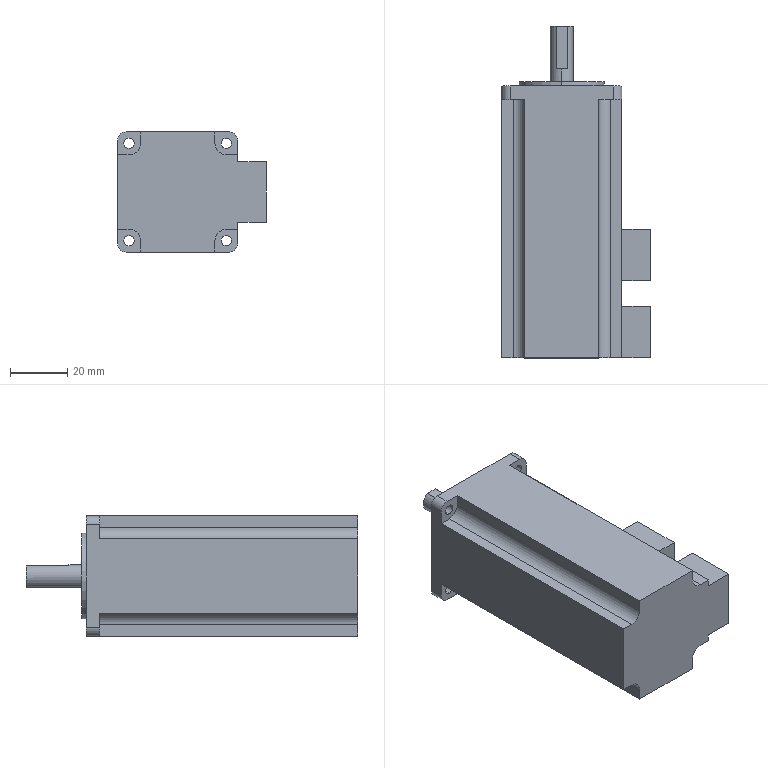Part | SolidWorks | features ICE 7, Fillet 2, Extrusion 1 | 1 solid | 51 faces | box 52 x 116 x 42 mm | volume 155076 mm3 | plane 31 | cylinder 20 | commonest cylinder face diameters 3.6 x8 8 x6 6 x4 30 x2
STEP:
#1=CARTESIAN_POINT('',(0.,101.,4.));
#2=VERTEX_POINT('',#1);
#3=CARTESIAN_POINT('',(1.936,101.,3.5));
#4=VERTEX_POINT('',#3);
#5=CARTESIAN_POINT('',(0.,101.,0.));
#6=DIRECTION('',(0.,1.,0.));
#7=DIRECTION('',(0.,0.,1.));
#8=AXIS2_PLACEMENT_3D('',#5,#6,#7);
#9=CIRCLE('',#8,4.);
#10=EDGE_CURVE('',#2,#4,#9,.T.);
#11=ORIENTED_EDGE('',*,*,#10,.F.);
#12=CARTESIAN_POINT('',(0.,96.5,4.));
#13=VERTEX_POINT('',#12);
#14=CARTESIAN_POINT('',(0.,116.,4.));
#15=DIRECTION('',(0.,-1.,0.));
#16=VECTOR('',#15,1000.);
#17=LINE('',#14,#16);
#18=EDGE_CURVE('',#2,#13,#17,.T.);
#19=ORIENTED_EDGE('',*,*,#18,.T.);
#20=CARTESIAN_POINT('',(0.,96.5,-4.));
#21=VERTEX_POINT('',#20);
#22=CARTESIAN_POINT('',(0.,96.5,0.));
#23=DIRECTION('',(0.,-1.,0.));
#24=DIRECTION('',(0.,0.,1.));
#25=AXIS2_PLACEMENT_3D('',#22,#23,#24);
#26=CIRCLE('',#25,4.);
#27=EDGE_CURVE('',#21,#13,#26,.T.);
#28=ORIENTED_EDGE('',*,*,#27,.F.);
#29=CARTESIAN_POINT('',(0.,116.,-4.));
#30=VERTEX_POINT('',#29);
#31=CARTESIAN_POINT('',(0.,116.,-4.));
#32=DIRECTION('',(0.,-1.,0.));
#33=VECTOR('',#32,1000.);
#34=LINE('',#31,#33);
#35=EDGE_CURVE('',#30,#21,#34,.T.);
#36=ORIENTED_EDGE('',*,*,#35,.F.);
#37=CARTESIAN_POINT('',(1.936,116.,3.5));
#38=VERTEX_POINT('',#37);
#39=CARTESIAN_POINT('',(0.,116.,0.));
#40=DIRECTION('',(0.,1.,0.));
#41=DIRECTION('',(0.,0.,1.));
#42=AXIS2_PLACEMENT_3D('',#39,#40,#41);
#43=CIRCLE('',#42,4.);
#44=EDGE_CURVE('',#38,#30,#43,.T.);
#45=ORIENTED_EDGE('',*,*,#44,.F.);
#46=CARTESIAN_POINT('',(1.936,116.,3.5));
#47=DIRECTION('',(0.,-1.,0.));
#48=VECTOR('',#47,1000.);
#49=LINE('',#46,#48);
#50=EDGE_CURVE('',#38,#4,#49,.T.);
#51=ORIENTED_EDGE('',*,*,#50,.T.);
#52=EDGE_LOOP('',(#11,#19,#28,#36,#45,#51));
#53=FACE_OUTER_BOUND('',#52,.T.);
#54=CARTESIAN_POINT('',(0.,116.,0.));
#55=DIRECTION('',(0.,-1.,0.));
#56=DIRECTION('',(0.,0.,-1.));
#57=AXIS2_PLACEMENT_3D('',#54,#55,#56);
#58=CYLINDRICAL_SURFACE('',#57,4.);
#59=ADVANCED_FACE('',(#53),#58,.T.);
#60=CARTESIAN_POINT('',(0.,96.5,15.));
#61=VERTEX_POINT('',#60);
#62=CARTESIAN_POINT('',(0.,96.5,-15.));
#63=VERTEX_POINT('',#62);
#64=CARTESIAN_POINT('',(0.,96.5,0.));
#65=DIRECTION('',(0.,1.,0.));
#66=DIRECTION('',(0.,0.,1.));
#67=AXIS2_PLACEMENT_3D('',#64,#65,#66);
#68=CIRCLE('',#67,15.);
#69=EDGE_CURVE('',#61,#63,#68,.T.);
#70=ORIENTED_EDGE('',*,*,#69,.F.);
#71=CARTESIAN_POINT('',(0.,95.,15.));
#72=VERTEX_POINT('',#71);
#73=CARTESIAN_POINT('',(0.,96.5,15.));
#74=DIRECTION('',(0.,-1.,0.));
#75=VECTOR('',#74,1000.);
#76=LINE('',#73,#75);
#77=EDGE_CURVE('',#61,#72,#76,.T.);
#78=ORIENTED_EDGE('',*,*,#77,.T.);
#79=CARTESIAN_POINT('',(0.,95.,-15.));
#80=VERTEX_POINT('',#79);
#81=CARTESIAN_POINT('',(0.,95.,0.));
#82=DIRECTION('',(0.,1.,0.));
#83=DIRECTION('',(0.,0.,-1.));
#84=AXIS2_PLACEMENT_3D('',#81,#82,#83);
#85=CIRCLE('',#84,15.);
#86=EDGE_CURVE('',#72,#80,#85,.T.);
#87=ORIENTED_EDGE('',*,*,#86,.T.);
#88=CARTESIAN_POINT('',(0.,96.5,-15.));
#89=DIRECTION('',(0.,-1.,0.));
#90=VECTOR('',#89,1000.);
#91=LINE('',#88,#90);
#92=EDGE_CURVE('',#63,#80,#91,.T.);
#93=ORIENTED_EDGE('',*,*,#92,.F.);
#94=EDGE_LOOP('',(#70,#78,#87,#93));
#95=FACE_OUTER_BOUND('',#94,.T.);
#96=CARTESIAN_POINT('',(0.,96.5,0.));
#97=DIRECTION('',(0.,-1.,0.));
#98=DIRECTION('',(0.,0.,-1.));
#99=AXIS2_PLACEMENT_3D('',#96,#97,#98);
#100=CYLINDRICAL_SURFACE('',#99,15.);
#101=ADVANCED_FACE('',(#95),#100,.T.);
#102=CARTESIAN_POINT('',(17.,90.2,15.2));
#103=VERTEX_POINT('',#102);
#104=CARTESIAN_POINT('',(17.,90.2,18.8));
#105=VERTEX_POINT('',#104);
#106=CARTESIAN_POINT('',(17.,90.2,17.));
#107=DIRECTION('',(0.,1.,0.));
#108=DIRECTION('',(0.,0.,1.));
#109=AXIS2_PLACEMENT_3D('',#106,#107,#108);
#110=CIRCLE('',#109,1.8);
#111=EDGE_CURVE('',#103,#105,#110,.T.);
#112=ORIENTED_EDGE('',*,*,#111,.F.);
#113=CARTESIAN_POINT('',(17.,95.,15.2));
#114=VERTEX_POINT('',#113);
#115=CARTESIAN_POINT('',(17.,90.2,15.2));
#116=DIRECTION('',(0.,1.,0.));
#117=VECTOR('',#116,1000.);
#118=LINE('',#115,#117);
#119=EDGE_CURVE('',#103,#114,#118,.T.);
#120=ORIENTED_EDGE('',*,*,#119,.T.);
#121=CARTESIAN_POINT('',(17.,95.,18.8));
#122=VERTEX_POINT('',#121);
#123=CARTESIAN_POINT('',(17.,95.,17.));
#124=DIRECTION('',(0.,1.,0.));
#125=DIRECTION('',(0.,0.,1.));
#126=AXIS2_PLACEMENT_3D('',#123,#124,#125);
#127=CIRCLE('',#126,1.8);
#128=EDGE_CURVE('',#114,#122,#127,.T.);
#129=ORIENTED_EDGE('',*,*,#128,.T.);
#130=CARTESIAN_POINT('',(17.,90.2,18.8));
#131=DIRECTION('',(0.,1.,0.));
#132=VECTOR('',#131,1000.);
#133=LINE('',#130,#132);
#134=EDGE_CURVE('',#105,#122,#133,.T.);
#135=ORIENTED_EDGE('',*,*,#134,.F.);
#136=EDGE_LOOP('',(#112,#120,#129,#135));
#137=FACE_OUTER_BOUND('',#136,.T.);
#138=CARTESIAN_POINT('',(17.,90.2,17.));
#139=DIRECTION('',(0.,1.,0.));
#140=DIRECTION('',(0.,0.,1.));
#141=AXIS2_PLACEMENT_3D('',#138,#139,#140);
#142=CYLINDRICAL_SURFACE('',#141,1.8);
#143=ADVANCED_FACE('',(#137),#142,.F.);
#144=CARTESIAN_POINT('',(-17.,90.2,15.2));
#145=VERTEX_POINT('',#144);
#146=CARTESIAN_POINT('',(-17.,90.2,18.8));
#147=VERTEX_POINT('',#146);
#148=CARTESIAN_POINT('',(-17.,90.2,17.));
#149=DIRECTION('',(0.,1.,0.));
#150=DIRECTION('',(0.,0.,1.));
#151=AXIS2_PLACEMENT_3D('',#148,#149,#150);
#152=CIRCLE('',#151,1.8);
#153=EDGE_CURVE('',#145,#147,#152,.T.);
#154=ORIENTED_EDGE('',*,*,#153,.F.);
#155=CARTESIAN_POINT('',(-17.,95.,15.2));
#156=VERTEX_POINT('',#155);
#157=CARTESIAN_POINT('',(-17.,90.2,15.2));
#158=DIRECTION('',(0.,1.,0.));
#159=VECTOR('',#158,1000.);
#160=LINE('',#157,#159);
#161=EDGE_CURVE('',#145,#156,#160,.T.);
#162=ORIENTED_EDGE('',*,*,#161,.T.);
#163=CARTESIAN_POINT('',(-17.,95.,18.8));
#164=VERTEX_POINT('',#163);
#165=CARTESIAN_POINT('',(-17.,95.,17.));
#166=DIRECTION('',(0.,1.,0.));
#167=DIRECTION('',(0.,0.,1.));
#168=AXIS2_PLACEMENT_3D('',#165,#166,#167);
#169=CIRCLE('',#168,1.8);
#170=EDGE_CURVE('',#156,#164,#169,.T.);
#171=ORIENTED_EDGE('',*,*,#170,.T.);
#172=CARTESIAN_POINT('',(-17.,90.2,18.8));
#173=DIRECTION('',(0.,1.,0.));
#174=VECTOR('',#173,1000.);
#175=LINE('',#172,#174);
#176=EDGE_CURVE('',#147,#164,#175,.T.);
#177=ORIENTED_EDGE('',*,*,#176,.F.);
#178=EDGE_LOOP('',(#154,#162,#171,#177));
#179=FACE_OUTER_BOUND('',#178,.T.);
#180=CARTESIAN_POINT('',(-17.,90.2,17.));
#181=DIRECTION('',(0.,1.,0.));
#182=DIRECTION('',(0.,0.,1.));
#183=AXIS2_PLACEMENT_3D('',#180,#181,#182);
#184=CYLINDRICAL_SURFACE('',#183,1.8);
#185=ADVANCED_FACE('',(#179),#184,.F.);
#186=CARTESIAN_POINT('',(17.,90.2,-18.8));
#187=VERTEX_POINT('',#186);
#188=CARTESIAN_POINT('',(17.,90.2,-15.2));
#189=VERTEX_POINT('',#188);
#190=CARTESIAN_POINT('',(17.,90.2,-17.));
#191=DIRECTION('',(0.,1.,0.));
#192=DIRECTION('',(0.,0.,1.));
#193=AXIS2_PLACEMENT_3D('',#190,#191,#192);
#194=CIRCLE('',#193,1.8);
#195=EDGE_CURVE('',#187,#189,#194,.T.);
#196=ORIENTED_EDGE('',*,*,#195,.F.);
#197=CARTESIAN_POINT('',(17.,95.,-18.8));
#198=VERTEX_POINT('',#197);
#199=CARTESIAN_POINT('',(17.,90.2,-18.8));
#200=DIRECTION('',(0.,1.,0.));
#201=VECTOR('',#200,1000.);
#202=LINE('',#199,#201);
#203=EDGE_CURVE('',#187,#198,#202,.T.);
#204=ORIENTED_EDGE('',*,*,#203,.T.);
#205=CARTESIAN_POINT('',(17.,95.,-15.2));
#206=VERTEX_POINT('',#205);
#207=CARTESIAN_POINT('',(17.,95.,-17.));
#208=DIRECTION('',(0.,1.,0.));
#209=DIRECTION('',(0.,0.,1.));
#210=AXIS2_PLACEMENT_3D('',#207,#208,#209);
#211=CIRCLE('',#210,1.8);
#212=EDGE_CURVE('',#198,#206,#211,.T.);
#213=ORIENTED_EDGE('',*,*,#212,.T.);
#214=CARTESIAN_POINT('',(17.,90.2,-15.2));
#215=DIRECTION('',(0.,1.,0.));
#216=VECTOR('',#215,1000.);
#217=LINE('',#214,#216);
#218=EDGE_CURVE('',#189,#206,#217,.T.);
#219=ORIENTED_EDGE('',*,*,#218,.F.);
#220=EDGE_LOOP('',(#196,#204,#213,#219));
#221=FACE_OUTER_BOUND('',#220,.T.);
#222=CARTESIAN_POINT('',(17.,90.2,-17.));
#223=DIRECTION('',(0.,1.,0.));
#224=DIRECTION('',(0.,0.,1.));
#225=AXIS2_PLACEMENT_3D('',#222,#223,#224);
#226=CYLINDRICAL_SURFACE('',#225,1.8);
#227=ADVANCED_FACE('',(#221),#226,.F.);
#228=CARTESIAN_POINT('',(-17.,90.2,-18.8));
#229=VERTEX_POINT('',#228);
#230=CARTESIAN_POINT('',(-17.,90.2,-15.2));
#231=VERTEX_POINT('',#230);
#232=CARTESIAN_POINT('',(-17.,90.2,-17.));
#233=DIRECTION('',(0.,1.,0.));
#234=DIRECTION('',(0.,0.,1.));
#235=AXIS2_PLACEMENT_3D('',#232,#233,#234);
#236=CIRCLE('',#235,1.8);
#237=EDGE_CURVE('',#229,#231,#236,.T.);
#238=ORIENTED_EDGE('',*,*,#237,.F.);
#239=CARTESIAN_POINT('',(-17.,95.,-18.8));
#240=VERTEX_POINT('',#239);
#241=CARTESIAN_POINT('',(-17.,90.2,-18.8));
#242=DIRECTION('',(0.,1.,0.));
#243=VECTOR('',#242,1000.);
#244=LINE('',#241,#243);
#245=EDGE_CURVE('',#229,#240,#244,.T.);
#246=ORIENTED_EDGE('',*,*,#245,.T.);
#247=CARTESIAN_POINT('',(-17.,95.,-15.2));
#248=VERTEX_POINT('',#247);
#249=CARTESIAN_POINT('',(-17.,95.,-17.));
#250=DIRECTION('',(0.,1.,0.));
#251=DIRECTION('',(0.,0.,1.));
#252=AXIS2_PLACEMENT_3D('',#249,#250,#251);
#253=CIRCLE('',#252,1.8);
#254=EDGE_CURVE('',#240,#248,#253,.T.);
#255=ORIENTED_EDGE('',*,*,#254,.T.);
#256=CARTESIAN_POINT('',(-17.,90.2,-15.2));
#257=DIRECTION('',(0.,1.,0.));
#258=VECTOR('',#257,1000.);
#259=LINE('',#256,#258);
#260=EDGE_CURVE('',#231,#248,#259,.T.);
#261=ORIENTED_EDGE('',*,*,#260,.F.);
#262=EDGE_LOOP('',(#238,#246,#255,#261));
#263=FACE_OUTER_BOUND('',#262,.T.);
#264=CARTESIAN_POINT('',(-17.,90.2,-17.));
#265=DIRECTION('',(0.,1.,0.));
#266=DIRECTION('',(0.,0.,1.));
#267=AXIS2_PLACEMENT_3D('',#264,#265,#266);
#268=CYLINDRICAL_SURFACE('',#267,1.8);
#269=ADVANCED_FACE('',(#263),#268,.F.);
#270=CARTESIAN_POINT('',(21.,0.,-10.5));
#271=VERTEX_POINT('',#270);
#272=CARTESIAN_POINT('',(21.,18.,-10.5));
#273=VERTEX_POINT('',#272);
#274=CARTESIAN_POINT('',(21.,0.,-10.5));
#275=DIRECTION('',(0.,1.,0.));
#276=VECTOR('',#275,1000.);
#277=LINE('',#274,#276);
#278=EDGE_CURVE('',#271,#273,#277,.T.);
#279=ORIENTED_EDGE('',*,*,#278,.F.);
#280=CARTESIAN_POINT('',(21.,0.,-13.));
#281=VERTEX_POINT('',#280);
#282=CARTESIAN_POINT('',(21.,0.,21.));
#283=DIRECTION('',(0.,0.,-1.));
#284=VECTOR('',#283,1000.);
#285=LINE('',#282,#284);
#286=EDGE_CURVE('',#271,#281,#285,.T.);
#287=ORIENTED_EDGE('',*,*,#286,.T.);
#288=CARTESIAN_POINT('',(21.,90.2,-13.));
#289=VERTEX_POINT('',#288);
#290=CARTESIAN_POINT('',(21.,106.314,-13.));
#291=DIRECTION('',(0.,-1.,0.));
#292=VECTOR('',#291,1000.);
#293=LINE('',#290,#292);
#294=EDGE_CURVE('',#289,#281,#293,.T.);
#295=ORIENTED_EDGE('',*,*,#294,.F.);
#296=CARTESIAN_POINT('',(21.,90.2,-18.));
#297=VERTEX_POINT('',#296);
#298=CARTESIAN_POINT('',(21.,90.2,-21.));
#299=DIRECTION('',(0.,0.,-1.));
#300=VECTOR('',#299,1000.);
#301=LINE('',#298,#300);
#302=EDGE_CURVE('',#289,#297,#301,.T.);
#303=ORIENTED_EDGE('',*,*,#302,.T.);
#304=CARTESIAN_POINT('',(21.,95.,-18.));
#305=VERTEX_POINT('',#304);
#306=CARTESIAN_POINT('',(21.,95.,-18.));
#307=DIRECTION('',(0.,1.,0.));
#308=VECTOR('',#307,1000.);
#309=LINE('',#306,#308);
#310=EDGE_CURVE('',#297,#305,#309,.T.);
#311=ORIENTED_EDGE('',*,*,#310,.T.);
#312=CARTESIAN_POINT('',(21.,95.,18.));
#313=VERTEX_POINT('',#312);
#314=CARTESIAN_POINT('',(21.,95.,21.));
#315=DIRECTION('',(0.,0.,-1.));
#316=VECTOR('',#315,1000.);
#317=LINE('',#314,#316);
#318=EDGE_CURVE('',#313,#305,#317,.T.);
#319=ORIENTED_EDGE('',*,*,#318,.F.);
#320=CARTESIAN_POINT('',(21.,90.2,18.));
#321=VERTEX_POINT('',#320);
#322=CARTESIAN_POINT('',(21.,95.,18.));
#323=DIRECTION('',(0.,-1.,0.));
#324=VECTOR('',#323,1000.);
#325=LINE('',#322,#324);
#326=EDGE_CURVE('',#313,#321,#325,.T.);
#327=ORIENTED_EDGE('',*,*,#326,.T.);
#328=CARTESIAN_POINT('',(21.,90.2,13.));
#329=VERTEX_POINT('',#328);
#330=CARTESIAN_POINT('',(21.,90.2,21.));
#331=DIRECTION('',(0.,0.,-1.));
#332=VECTOR('',#331,1000.);
#333=LINE('',#330,#332);
#334=EDGE_CURVE('',#321,#329,#333,.T.);
#335=ORIENTED_EDGE('',*,*,#334,.T.);
#336=CARTESIAN_POINT('',(21.,0.,13.));
#337=VERTEX_POINT('',#336);
#338=CARTESIAN_POINT('',(21.,106.314,13.));
#339=DIRECTION('',(0.,-1.,0.));
#340=VECTOR('',#339,1000.);
#341=LINE('',#338,#340);
#342=EDGE_CURVE('',#329,#337,#341,.T.);
#343=ORIENTED_EDGE('',*,*,#342,.T.);
#344=CARTESIAN_POINT('',(21.,0.,10.5));
#345=VERTEX_POINT('',#344);
#346=CARTESIAN_POINT('',(21.,0.,21.));
#347=DIRECTION('',(0.,0.,-1.));
#348=VECTOR('',#347,1000.);
#349=LINE('',#346,#348);
#350=EDGE_CURVE('',#337,#345,#349,.T.);
#351=ORIENTED_EDGE('',*,*,#350,.T.);
#352=CARTESIAN_POINT('',(21.,18.,10.5));
#353=VERTEX_POINT('',#352);
#354=CARTESIAN_POINT('',(21.,0.,10.5));
#355=DIRECTION('',(0.,-1.,0.));
#356=VECTOR('',#355,1000.);
#357=LINE('',#354,#356);
#358=EDGE_CURVE('',#353,#345,#357,.T.);
#359=ORIENTED_EDGE('',*,*,#358,.F.);
#360=CARTESIAN_POINT('',(21.,18.,-10.5));
#361=DIRECTION('',(0.,0.,1.));
#362=VECTOR('',#361,1000.);
#363=LINE('',#360,#362);
#364=EDGE_CURVE('',#273,#353,#363,.T.);
#365=ORIENTED_EDGE('',*,*,#364,.F.);
#366=EDGE_LOOP('',(#279,#287,#295,#303,#311,#319,#327,#335,#343,#351,#359,#365));
#367=FACE_OUTER_BOUND('',#366,.T.);
#368=CARTESIAN_POINT('',(21.,45.,10.5));
#369=VERTEX_POINT('',#368);
#370=CARTESIAN_POINT('',(21.,27.,10.5));
#371=VERTEX_POINT('',#370);
#372=CARTESIAN_POINT('',(21.,45.,10.5));
#373=DIRECTION('',(0.,-1.,0.));
#374=VECTOR('',#373,1000.);
#375=LINE('',#372,#374);
#376=EDGE_CURVE('',#369,#371,#375,.T.);
#377=ORIENTED_EDGE('',*,*,#376,.F.);
#378=CARTESIAN_POINT('',(21.,45.,-10.5));
#379=VERTEX_POINT('',#378);
#380=CARTESIAN_POINT('',(21.,45.,10.5));
#381=DIRECTION('',(0.,0.,1.));
#382=VECTOR('',#381,1000.);
#383=LINE('',#380,#382);
#384=EDGE_CURVE('',#379,#369,#383,.T.);
#385=ORIENTED_EDGE('',*,*,#384,.F.);
#386=CARTESIAN_POINT('',(21.,27.,-10.5));
#387=VERTEX_POINT('',#386);
#388=CARTESIAN_POINT('',(21.,45.,-10.5));
#389=DIRECTION('',(0.,1.,0.));
#390=VECTOR('',#389,1000.);
#391=LINE('',#388,#390);
#392=EDGE_CURVE('',#387,#379,#391,.T.);
#393=ORIENTED_EDGE('',*,*,#392,.F.);
#394=CARTESIAN_POINT('',(21.,27.,10.5));
#395=DIRECTION('',(0.,0.,-1.));
#396=VECTOR('',#395,1000.);
#397=LINE('',#394,#396);
#398=EDGE_CURVE('',#371,#387,#397,.T.);
#399=ORIENTED_EDGE('',*,*,#398,.F.);
#400=EDGE_LOOP('',(#377,#385,#393,#399));
#401=FACE_BOUND('',#400,.T.);
#402=CARTESIAN_POINT('',(21.,95.,21.));
#403=DIRECTION('',(-1.,0.,0.));
#404=DIRECTION('',(0.,0.,1.));
#405=AXIS2_PLACEMENT_3D('',#402,#403,#404);
#406=PLANE('',#405);
#407=ADVANCED_FACE('',(#367,#401),#406,.F.);
#408=CARTESIAN_POINT('',(0.,96.5,0.));
#409=DIRECTION('',(0.,1.,0.));
#410=DIRECTION('',(0.,0.,1.));
#411=AXIS2_PLACEMENT_3D('',#408,#409,#410);
#412=CIRCLE('',#411,15.);
#413=EDGE_CURVE('',#63,#61,#412,.T.);
#414=ORIENTED_EDGE('',*,*,#413,.T.);
#415=ORIENTED_EDGE('',*,*,#69,.T.);
#416=EDGE_LOOP('',(#414,#415));
#417=FACE_OUTER_BOUND('',#416,.T.);
#418=ORIENTED_EDGE('',*,*,#27,.T.);
#419=CARTESIAN_POINT('',(0.,96.5,0.));
#420=DIRECTION('',(0.,-1.,0.));
#421=DIRECTION('',(0.,0.,1.));
#422=AXIS2_PLACEMENT_3D('',#419,#420,#421);
#423=CIRCLE('',#422,4.);
#424=EDGE_CURVE('',#13,#21,#423,.T.);
#425=ORIENTED_EDGE('',*,*,#424,.T.);
#426=EDGE_LOOP('',(#418,#425));
#427=FACE_BOUND('',#426,.T.);
#428=CARTESIAN_POINT('',(0.,96.5,0.));
#429=DIRECTION('',(0.,1.,0.));
#430=DIRECTION('',(0.,0.,1.));
#431=AXIS2_PLACEMENT_3D('',#428,#429,#430);
#432=PLANE('',#431);
#433=ADVANCED_FACE('',(#417,#427),#432,.T.);
#434=CARTESIAN_POINT('',(18.,95.,-21.));
#435=VERTEX_POINT('',#434);
#436=CARTESIAN_POINT('',(-18.,95.,-21.));
#437=VERTEX_POINT('',#436);
#438=CARTESIAN_POINT('',(-21.,95.,-21.));
#439=DIRECTION('',(-1.,0.,0.));
#440=VECTOR('',#439,1000.);
#441=LINE('',#438,#440);
#442=EDGE_CURVE('',#435,#437,#441,.T.);
#443=ORIENTED_EDGE('',*,*,#442,.T.);
#444=CARTESIAN_POINT('',(-21.,95.,-18.));
#445=VERTEX_POINT('',#444);
#446=CARTESIAN_POINT('',(-18.,95.,-18.));
#447=DIRECTION('',(0.,1.,0.));
#448=DIRECTION('',(0.,0.,-1.));
#449=AXIS2_PLACEMENT_3D('',#446,#447,#448);
#450=CIRCLE('',#449,3.);
#451=EDGE_CURVE('',#437,#445,#450,.T.);
#452=ORIENTED_EDGE('',*,*,#451,.T.);
#453=CARTESIAN_POINT('',(-21.,95.,18.));
#454=VERTEX_POINT('',#453);
#455=CARTESIAN_POINT('',(-21.,95.,21.));
#456=DIRECTION('',(0.,0.,1.));
#457=VECTOR('',#456,1000.);
#458=LINE('',#455,#457);
#459=EDGE_CURVE('',#445,#454,#458,.T.);
#460=ORIENTED_EDGE('',*,*,#459,.T.);
#461=CARTESIAN_POINT('',(-18.,95.,21.));
#462=VERTEX_POINT('',#461);
#463=CARTESIAN_POINT('',(-18.,95.,18.));
#464=DIRECTION('',(0.,1.,0.));
#465=DIRECTION('',(0.,0.,-1.));
#466=AXIS2_PLACEMENT_3D('',#463,#464,#465);
#467=CIRCLE('',#466,3.);
#468=EDGE_CURVE('',#454,#462,#467,.T.);
#469=ORIENTED_EDGE('',*,*,#468,.T.);
#470=CARTESIAN_POINT('',(18.,95.,21.));
#471=VERTEX_POINT('',#470);
#472=CARTESIAN_POINT('',(-21.,95.,21.));
#473=DIRECTION('',(1.,0.,0.));
#474=VECTOR('',#473,1000.);
#475=LINE('',#472,#474);
#476=EDGE_CURVE('',#462,#471,#475,.T.);
#477=ORIENTED_EDGE('',*,*,#476,.T.);
#478=CARTESIAN_POINT('',(18.,95.,18.));
#479=DIRECTION('',(0.,1.,0.));
#480=DIRECTION('',(0.,0.,-1.));
#481=AXIS2_PLACEMENT_3D('',#478,#479,#480);
#482=CIRCLE('',#481,3.);
#483=EDGE_CURVE('',#471,#313,#482,.T.);
#484=ORIENTED_EDGE('',*,*,#483,.T.);
#485=ORIENTED_EDGE('',*,*,#318,.T.);
#486=CARTESIAN_POINT('',(18.,95.,-18.));
#487=DIRECTION('',(0.,1.,0.));
#488=DIRECTION('',(0.,0.,-1.));
#489=AXIS2_PLACEMENT_3D('',#486,#487,#488);
#490=CIRCLE('',#489,3.);
#491=EDGE_CURVE('',#305,#435,#490,.T.);
#492=ORIENTED_EDGE('',*,*,#491,.T.);
#493=EDGE_LOOP('',(#443,#452,#460,#469,#477,#484,#485,#492));
#494=FACE_OUTER_BOUND('',#493,.T.);
#495=CARTESIAN_POINT('',(-17.,95.,-17.));
#496=DIRECTION('',(0.,1.,0.));
#497=DIRECTION('',(0.,0.,1.));
#498=AXIS2_PLACEMENT_3D('',#495,#496,#497);
#499=CIRCLE('',#498,1.8);
#500=EDGE_CURVE('',#248,#240,#499,.T.);
#501=ORIENTED_EDGE('',*,*,#500,.F.);
#502=ORIENTED_EDGE('',*,*,#254,.F.);
#503=EDGE_LOOP('',(#501,#502));
#504=FACE_BOUND('',#503,.T.);
#505=CARTESIAN_POINT('',(17.,95.,-17.));
#506=DIRECTION('',(0.,1.,0.));
#507=DIRECTION('',(0.,0.,1.));
#508=AXIS2_PLACEMENT_3D('',#505,#506,#507);
#509=CIRCLE('',#508,1.8);
#510=EDGE_CURVE('',#206,#198,#509,.T.);
#511=ORIENTED_EDGE('',*,*,#510,.F.);
#512=ORIENTED_EDGE('',*,*,#212,.F.);
#513=EDGE_LOOP('',(#511,#512));
#514=FACE_BOUND('',#513,.T.);
#515=CARTESIAN_POINT('',(-17.,95.,17.));
#516=DIRECTION('',(0.,1.,0.));
#517=DIRECTION('',(0.,0.,1.));
#518=AXIS2_PLACEMENT_3D('',#515,#516,#517);
#519=CIRCLE('',#518,1.8);
#520=EDGE_CURVE('',#164,#156,#519,.T.);
#521=ORIENTED_EDGE('',*,*,#520,.F.);
#522=ORIENTED_EDGE('',*,*,#170,.F.);
#523=EDGE_LOOP('',(#521,#522));
#524=FACE_BOUND('',#523,.T.);
#525=CARTESIAN_POINT('',(17.,95.,17.));
#526=DIRECTION('',(0.,1.,0.));
#527=DIRECTION('',(0.,0.,1.));
#528=AXIS2_PLACEMENT_3D('',#525,#526,#527);
#529=CIRCLE('',#528,1.8);
#530=EDGE_CURVE('',#122,#114,#529,.T.);
#531=ORIENTED_EDGE('',*,*,#530,.F.);
#532=ORIENTED_EDGE('',*,*,#128,.F.);
#533=EDGE_LOOP('',(#531,#532));
#534=FACE_BOUND('',#533,.T.);
#535=CARTESIAN_POINT('',(0.,95.,0.));
#536=DIRECTION('',(0.,1.,0.));
#537=DIRECTION('',(0.,0.,-1.));
#538=AXIS2_PLACEMENT_3D('',#535,#536,#537);
#539=CIRCLE('',#538,15.);
#540=EDGE_CURVE('',#80,#72,#539,.T.);
#541=ORIENTED_EDGE('',*,*,#540,.F.);
#542=ORIENTED_EDGE('',*,*,#86,.F.);
#543=EDGE_LOOP('',(#541,#542));
#544=FACE_BOUND('',#543,.T.);
#545=CARTESIAN_POINT('',(21.,95.,-21.));
#546=DIRECTION('',(0.,-1.,0.));
#547=DIRECTION('',(0.,0.,-1.));
#548=AXIS2_PLACEMENT_3D('',#545,#546,#547);
#549=PLANE('',#548);
#550=ADVANCED_FACE('',(#494,#504,#514,#524,#534,#544),#549,.F.);
#551=CARTESIAN_POINT('',(-13.,90.2,-21.));
#552=VERTEX_POINT('',#551);
#553=CARTESIAN_POINT('',(-18.,90.2,-21.));
#554=VERTEX_POINT('',#553);
#555=CARTESIAN_POINT('',(-21.,90.2,-21.));
#556=DIRECTION('',(-1.,0.,0.));
#557=VECTOR('',#556,1000.);
#558=LINE('',#555,#557);
#559=EDGE_CURVE('',#552,#554,#558,.T.);
#560=ORIENTED_EDGE('',*,*,#559,.T.);
#561=CARTESIAN_POINT('',(-18.,95.,-21.));
#562=DIRECTION('',(0.,1.,0.));
#563=VECTOR('',#562,1000.);
#564=LINE('',#561,#563);
#565=EDGE_CURVE('',#554,#437,#564,.T.);
#566=ORIENTED_EDGE('',*,*,#565,.T.);
#567=ORIENTED_EDGE('',*,*,#442,.F.);
#568=CARTESIAN_POINT('',(18.,90.2,-21.));
#569=VERTEX_POINT('',#568);
#570=CARTESIAN_POINT('',(18.,95.,-21.));
#571=DIRECTION('',(0.,-1.,0.));
#572=VECTOR('',#571,1000.);
#573=LINE('',#570,#572);
#574=EDGE_CURVE('',#435,#569,#573,.T.);
#575=ORIENTED_EDGE('',*,*,#574,.T.);
#576=CARTESIAN_POINT('',(13.,90.2,-21.));
#577=VERTEX_POINT('',#576);
#578=CARTESIAN_POINT('',(21.,90.2,-21.));
#579=DIRECTION('',(-1.,0.,0.));
#580=VECTOR('',#579,1000.);
#581=LINE('',#578,#580);
#582=EDGE_CURVE('',#569,#577,#581,.T.);
#583=ORIENTED_EDGE('',*,*,#582,.T.);
#584=CARTESIAN_POINT('',(13.,0.,-21.));
#585=VERTEX_POINT('',#584);
#586=CARTESIAN_POINT('',(13.,106.314,-21.));
#587=DIRECTION('',(0.,-1.,0.));
#588=VECTOR('',#587,1000.);
#589=LINE('',#586,#588);
#590=EDGE_CURVE('',#577,#585,#589,.T.);
#591=ORIENTED_EDGE('',*,*,#590,.T.);
#592=CARTESIAN_POINT('',(-13.,0.,-21.));
#593=VERTEX_POINT('',#592);
#594=CARTESIAN_POINT('',(-21.,0.,-21.));
#595=DIRECTION('',(-1.,0.,0.));
#596=VECTOR('',#595,1000.);
#597=LINE('',#594,#596);
#598=EDGE_CURVE('',#585,#593,#597,.T.);
#599=ORIENTED_EDGE('',*,*,#598,.T.);
#600=CARTESIAN_POINT('',(-13.,106.314,-21.));
#601=DIRECTION('',(0.,-1.,0.));
#602=VECTOR('',#601,1000.);
#603=LINE('',#600,#602);
#604=EDGE_CURVE('',#552,#593,#603,.T.);
#605=ORIENTED_EDGE('',*,*,#604,.F.);
#606=EDGE_LOOP('',(#560,#566,#567,#575,#583,#591,#599,#605));
#607=FACE_OUTER_BOUND('',#606,.T.);
#608=CARTESIAN_POINT('',(-21.,95.,-21.));
#609=DIRECTION('',(0.,0.,1.));
#610=DIRECTION('',(1.,0.,0.));
#611=AXIS2_PLACEMENT_3D('',#608,#609,#610);
#612=PLANE('',#611);
#613=ADVANCED_FACE('',(#607),#612,.F.);
#614=ORIENTED_EDGE('',*,*,#459,.F.);
#615=CARTESIAN_POINT('',(-21.,90.2,-18.));
#616=VERTEX_POINT('',#615);
#617=CARTESIAN_POINT('',(-21.,95.,-18.));
#618=DIRECTION('',(0.,-1.,0.));
#619=VECTOR('',#618,1000.);
#620=LINE('',#617,#619);
#621=EDGE_CURVE('',#445,#616,#620,.T.);
#622=ORIENTED_EDGE('',*,*,#621,.T.);
#623=CARTESIAN_POINT('',(-21.,90.2,-13.));
#624=VERTEX_POINT('',#623);
#625=CARTESIAN_POINT('',(-21.,90.2,-21.));
#626=DIRECTION('',(0.,0.,1.));
#627=VECTOR('',#626,1000.);
#628=LINE('',#625,#627);
#629=EDGE_CURVE('',#616,#624,#628,.T.);
#630=ORIENTED_EDGE('',*,*,#629,.T.);
#631=CARTESIAN_POINT('',(-21.,0.,-13.));
#632=VERTEX_POINT('',#631);
#633=CARTESIAN_POINT('',(-21.,106.314,-13.));
#634=DIRECTION('',(0.,-1.,0.));
#635=VECTOR('',#634,1000.);
#636=LINE('',#633,#635);
#637=EDGE_CURVE('',#624,#632,#636,.T.);
#638=ORIENTED_EDGE('',*,*,#637,.T.);
#639=CARTESIAN_POINT('',(-21.,0.,13.));
#640=VERTEX_POINT('',#639);
#641=CARTESIAN_POINT('',(-21.,0.,21.));
#642=DIRECTION('',(0.,0.,1.));
#643=VECTOR('',#642,1000.);
#644=LINE('',#641,#643);
#645=EDGE_CURVE('',#632,#640,#644,.T.);
#646=ORIENTED_EDGE('',*,*,#645,.T.);
#647=CARTESIAN_POINT('',(-21.,90.2,13.));
#648=VERTEX_POINT('',#647);
#649=CARTESIAN_POINT('',(-21.,106.314,13.));
#650=DIRECTION('',(0.,-1.,0.));
#651=VECTOR('',#650,1000.);
#652=LINE('',#649,#651);
#653=EDGE_CURVE('',#648,#640,#652,.T.);
#654=ORIENTED_EDGE('',*,*,#653,.F.);
#655=CARTESIAN_POINT('',(-21.,90.2,18.));
#656=VERTEX_POINT('',#655);
#657=CARTESIAN_POINT('',(-21.,90.2,21.));
#658=DIRECTION('',(0.,0.,1.));
#659=VECTOR('',#658,1000.);
#660=LINE('',#657,#659);
#661=EDGE_CURVE('',#648,#656,#660,.T.);
#662=ORIENTED_EDGE('',*,*,#661,.T.);
#663=CARTESIAN_POINT('',(-21.,95.,18.));
#664=DIRECTION('',(0.,1.,0.));
#665=VECTOR('',#664,1000.);
#666=LINE('',#663,#665);
#667=EDGE_CURVE('',#656,#454,#666,.T.);
#668=ORIENTED_EDGE('',*,*,#667,.T.);
#669=EDGE_LOOP('',(#614,#622,#630,#638,#646,#654,#662,#668));
#670=FACE_OUTER_BOUND('',#669,.T.);
#671=CARTESIAN_POINT('',(-21.,95.,21.));
#672=DIRECTION('',(1.,0.,0.));
#673=DIRECTION('',(0.,0.,-1.));
#674=AXIS2_PLACEMENT_3D('',#671,#672,#673);
#675=PLANE('',#674);
#676=ADVANCED_FACE('',(#670),#675,.F.);
#677=ORIENTED_EDGE('',*,*,#476,.F.);
#678=CARTESIAN_POINT('',(-18.,90.2,21.));
#679=VERTEX_POINT('',#678);
#680=CARTESIAN_POINT('',(-18.,95.,21.));
#681=DIRECTION('',(0.,-1.,0.));
#682=VECTOR('',#681,1000.);
#683=LINE('',#680,#682);
#684=EDGE_CURVE('',#462,#679,#683,.T.);
#685=ORIENTED_EDGE('',*,*,#684,.T.);
#686=CARTESIAN_POINT('',(-13.,90.2,21.));
#687=VERTEX_POINT('',#686);
#688=CARTESIAN_POINT('',(-21.,90.2,21.));
#689=DIRECTION('',(1.,0.,0.));
#690=VECTOR('',#689,1000.);
#691=LINE('',#688,#690);
#692=EDGE_CURVE('',#679,#687,#691,.T.);
#693=ORIENTED_EDGE('',*,*,#692,.T.);
#694=CARTESIAN_POINT('',(-13.,0.,21.));
#695=VERTEX_POINT('',#694);
#696=CARTESIAN_POINT('',(-13.,106.314,21.));
#697=DIRECTION('',(0.,-1.,0.));
#698=VECTOR('',#697,1000.);
#699=LINE('',#696,#698);
#700=EDGE_CURVE('',#687,#695,#699,.T.);
#701=ORIENTED_EDGE('',*,*,#700,.T.);
#702=CARTESIAN_POINT('',(13.,0.,21.));
#703=VERTEX_POINT('',#702);
#704=CARTESIAN_POINT('',(-21.,0.,21.));
#705=DIRECTION('',(1.,0.,0.));
#706=VECTOR('',#705,1000.);
#707=LINE('',#704,#706);
#708=EDGE_CURVE('',#695,#703,#707,.T.);
#709=ORIENTED_EDGE('',*,*,#708,.T.);
#710=CARTESIAN_POINT('',(13.,90.2,21.));
#711=VERTEX_POINT('',#710);
#712=CARTESIAN_POINT('',(13.,106.314,21.));
#713=DIRECTION('',(0.,-1.,0.));
#714=VECTOR('',#713,1000.);
#715=LINE('',#712,#714);
#716=EDGE_CURVE('',#711,#703,#715,.T.);
#717=ORIENTED_EDGE('',*,*,#716,.F.);
#718=CARTESIAN_POINT('',(18.,90.2,21.));
#719=VERTEX_POINT('',#718);
#720=CARTESIAN_POINT('',(21.,90.2,21.));
#721=DIRECTION('',(1.,0.,0.));
#722=VECTOR('',#721,1000.);
#723=LINE('',#720,#722);
#724=EDGE_CURVE('',#711,#719,#723,.T.);
#725=ORIENTED_EDGE('',*,*,#724,.T.);
#726=CARTESIAN_POINT('',(18.,95.,21.));
#727=DIRECTION('',(0.,1.,0.));
#728=VECTOR('',#727,1000.);
#729=LINE('',#726,#728);
#730=EDGE_CURVE('',#719,#471,#729,.T.);
#731=ORIENTED_EDGE('',*,*,#730,.T.);
#732=EDGE_LOOP('',(#677,#685,#693,#701,#709,#717,#725,#731));
#733=FACE_OUTER_BOUND('',#732,.T.);
#734=CARTESIAN_POINT('',(-21.,95.,21.));
#735=DIRECTION('',(0.,0.,-1.));
#736=DIRECTION('',(-1.,0.,0.));
#737=AXIS2_PLACEMENT_3D('',#734,#735,#736);
#738=PLANE('',#737);
#739=ADVANCED_FACE('',(#733),#738,.F.);
#740=CARTESIAN_POINT('',(13.,0.,-17.));
#741=VERTEX_POINT('',#740);
#742=CARTESIAN_POINT('',(13.,0.,-21.));
#743=DIRECTION('',(0.,0.,-1.));
#744=VECTOR('',#743,1000.);
#745=LINE('',#742,#744);
#746=EDGE_CURVE('',#741,#585,#745,.T.);
#747=ORIENTED_EDGE('',*,*,#746,.F.);
#748=CARTESIAN_POINT('',(17.,0.,-13.));
#749=VERTEX_POINT('',#748);
#750=CARTESIAN_POINT('',(17.,0.,-17.));
#751=DIRECTION('',(0.,1.,0.));
#752=DIRECTION('',(0.,0.,-1.));
#753=AXIS2_PLACEMENT_3D('',#750,#751,#752);
#754=CIRCLE('',#753,4.);
#755=EDGE_CURVE('',#741,#749,#754,.T.);
#756=ORIENTED_EDGE('',*,*,#755,.T.);
#757=CARTESIAN_POINT('',(21.,0.,-13.));
#758=DIRECTION('',(-1.,0.,0.));
#759=VECTOR('',#758,1000.);
#760=LINE('',#757,#759);
#761=EDGE_CURVE('',#281,#749,#760,.T.);
#762=ORIENTED_EDGE('',*,*,#761,.F.);
#763=ORIENTED_EDGE('',*,*,#286,.F.);
#764=CARTESIAN_POINT('',(31.,0.,-10.5));
#765=VERTEX_POINT('',#764);
#766=CARTESIAN_POINT('',(31.,0.,-10.5));
#767=DIRECTION('',(-1.,0.,0.));
#768=VECTOR('',#767,1000.);
#769=LINE('',#766,#768);
#770=EDGE_CURVE('',#765,#271,#769,.T.);
#771=ORIENTED_EDGE('',*,*,#770,.F.);
#772=CARTESIAN_POINT('',(31.,0.,10.5));
#773=VERTEX_POINT('',#772);
#774=CARTESIAN_POINT('',(31.,0.,-10.5));
#775=DIRECTION('',(0.,0.,-1.));
#776=VECTOR('',#775,1000.);
#777=LINE('',#774,#776);
#778=EDGE_CURVE('',#773,#765,#777,.T.);
#779=ORIENTED_EDGE('',*,*,#778,.F.);
#780=CARTESIAN_POINT('',(31.,0.,10.5));
#781=DIRECTION('',(-1.,0.,0.));
#782=VECTOR('',#781,1000.);
#783=LINE('',#780,#782);
#784=EDGE_CURVE('',#773,#345,#783,.T.);
#785=ORIENTED_EDGE('',*,*,#784,.T.);
#786=ORIENTED_EDGE('',*,*,#350,.F.);
#787=CARTESIAN_POINT('',(17.,0.,13.));
#788=VERTEX_POINT('',#787);
#789=CARTESIAN_POINT('',(21.,0.,13.));
#790=DIRECTION('',(1.,0.,0.));
#791=VECTOR('',#790,1000.);
#792=LINE('',#789,#791);
#793=EDGE_CURVE('',#788,#337,#792,.T.);
#794=ORIENTED_EDGE('',*,*,#793,.F.);
#795=CARTESIAN_POINT('',(13.,0.,17.));
#796=VERTEX_POINT('',#795);
#797=CARTESIAN_POINT('',(17.,0.,17.));
#798=DIRECTION('',(0.,1.,0.));
#799=DIRECTION('',(0.,0.,-1.));
#800=AXIS2_PLACEMENT_3D('',#797,#798,#799);
#801=CIRCLE('',#800,4.);
#802=EDGE_CURVE('',#788,#796,#801,.T.);
#803=ORIENTED_EDGE('',*,*,#802,.T.);
#804=CARTESIAN_POINT('',(13.,0.,21.));
#805=DIRECTION('',(0.,0.,-1.));
#806=VECTOR('',#805,1000.);
#807=LINE('',#804,#806);
#808=EDGE_CURVE('',#703,#796,#807,.T.);
#809=ORIENTED_EDGE('',*,*,#808,.F.);
#810=ORIENTED_EDGE('',*,*,#708,.F.);
#811=CARTESIAN_POINT('',(-13.,0.,17.));
#812=VERTEX_POINT('',#811);
#813=CARTESIAN_POINT('',(-13.,0.,21.));
#814=DIRECTION('',(0.,0.,1.));
#815=VECTOR('',#814,1000.);
#816=LINE('',#813,#815);
#817=EDGE_CURVE('',#812,#695,#816,.T.);
#818=ORIENTED_EDGE('',*,*,#817,.F.);
#819=CARTESIAN_POINT('',(-17.,0.,13.));
#820=VERTEX_POINT('',#819);
#821=CARTESIAN_POINT('',(-17.,0.,17.));
#822=DIRECTION('',(0.,1.,0.));
#823=DIRECTION('',(0.,0.,-1.));
#824=AXIS2_PLACEMENT_3D('',#821,#822,#823);
#825=CIRCLE('',#824,4.);
#826=EDGE_CURVE('',#812,#820,#825,.T.);
#827=ORIENTED_EDGE('',*,*,#826,.T.);
#828=CARTESIAN_POINT('',(-21.,0.,13.));
#829=DIRECTION('',(1.,0.,0.));
#830=VECTOR('',#829,1000.);
#831=LINE('',#828,#830);
#832=EDGE_CURVE('',#640,#820,#831,.T.);
#833=ORIENTED_EDGE('',*,*,#832,.F.);
#834=ORIENTED_EDGE('',*,*,#645,.F.);
#835=CARTESIAN_POINT('',(-17.,0.,-13.));
#836=VERTEX_POINT('',#835);
#837=CARTESIAN_POINT('',(-21.,0.,-13.));
#838=DIRECTION('',(-1.,0.,0.));
#839=VECTOR('',#838,1000.);
#840=LINE('',#837,#839);
#841=EDGE_CURVE('',#836,#632,#840,.T.);
#842=ORIENTED_EDGE('',*,*,#841,.F.);
#843=CARTESIAN_POINT('',(-13.,0.,-17.));
#844=VERTEX_POINT('',#843);
#845=CARTESIAN_POINT('',(-17.,0.,-17.));
#846=DIRECTION('',(0.,1.,0.));
#847=DIRECTION('',(0.,0.,-1.));
#848=AXIS2_PLACEMENT_3D('',#845,#846,#847);
#849=CIRCLE('',#848,4.);
#850=EDGE_CURVE('',#836,#844,#849,.T.);
#851=ORIENTED_EDGE('',*,*,#850,.T.);
#852=CARTESIAN_POINT('',(-13.,0.,-21.));
#853=DIRECTION('',(0.,0.,1.));
#854=VECTOR('',#853,1000.);
#855=LINE('',#852,#854);
#856=EDGE_CURVE('',#593,#844,#855,.T.);
#857=ORIENTED_EDGE('',*,*,#856,.F.);
#858=ORIENTED_EDGE('',*,*,#598,.F.);
#859=EDGE_LOOP('',(#747,#756,#762,#763,#771,#779,#785,#786,#794,#803,#809,#810,#818,#827,#833,#834,#842,#851,#857,#858));
#860=FACE_OUTER_BOUND('',#859,.T.);
#861=CARTESIAN_POINT('',(21.,0.,-21.));
#862=DIRECTION('',(0.,-1.,0.));
#863=DIRECTION('',(0.,0.,-1.));
#864=AXIS2_PLACEMENT_3D('',#861,#862,#863);
#865=PLANE('',#864);
#866=ADVANCED_FACE('',(#860),#865,.T.);
#867=CARTESIAN_POINT('',(-13.,90.2,17.));
#868=VERTEX_POINT('',#867);
#869=CARTESIAN_POINT('',(-13.,90.2,21.));
#870=DIRECTION('',(0.,0.,-1.));
#871=VECTOR('',#870,1000.);
#872=LINE('',#869,#871);
#873=EDGE_CURVE('',#687,#868,#872,.T.);
#874=ORIENTED_EDGE('',*,*,#873,.T.);
#875=CARTESIAN_POINT('',(-13.,0.,17.));
#876=DIRECTION('',(0.,-1.,0.));
#877=VECTOR('',#876,1000.);
#878=LINE('',#875,#877);
#879=EDGE_CURVE('',#868,#812,#878,.T.);
#880=ORIENTED_EDGE('',*,*,#879,.T.);
#881=ORIENTED_EDGE('',*,*,#817,.T.);
#882=ORIENTED_EDGE('',*,*,#700,.F.);
#883=EDGE_LOOP('',(#874,#880,#881,#882));
#884=FACE_OUTER_BOUND('',#883,.T.);
#885=CARTESIAN_POINT('',(-13.,106.314,21.));
#886=DIRECTION('',(1.,0.,0.));
#887=DIRECTION('',(0.,0.,-1.));
#888=AXIS2_PLACEMENT_3D('',#885,#886,#887);
#889=PLANE('',#888);
#890=ADVANCED_FACE('',(#884),#889,.F.);
#891=ORIENTED_EDGE('',*,*,#832,.T.);
#892=CARTESIAN_POINT('',(-17.,90.2,13.));
#893=VERTEX_POINT('',#892);
#894=CARTESIAN_POINT('',(-17.,90.2,13.));
#895=DIRECTION('',(0.,1.,0.));
#896=VECTOR('',#895,1000.);
#897=LINE('',#894,#896);
#898=EDGE_CURVE('',#820,#893,#897,.T.);
#899=ORIENTED_EDGE('',*,*,#898,.T.);
#900=CARTESIAN_POINT('',(-21.,90.2,13.));
#901=DIRECTION('',(-1.,0.,0.));
#902=VECTOR('',#901,1000.);
#903=LINE('',#900,#902);
#904=EDGE_CURVE('',#893,#648,#903,.T.);
#905=ORIENTED_EDGE('',*,*,#904,.T.);
#906=ORIENTED_EDGE('',*,*,#653,.T.);
#907=EDGE_LOOP('',(#891,#899,#905,#906));
#908=FACE_OUTER_BOUND('',#907,.T.);
#909=CARTESIAN_POINT('',(-21.,106.314,13.));
#910=DIRECTION('',(0.,0.,-1.));
#911=DIRECTION('',(-1.,0.,0.));
#912=AXIS2_PLACEMENT_3D('',#909,#910,#911);
#913=PLANE('',#912);
#914=ADVANCED_FACE('',(#908),#913,.F.);
#915=CARTESIAN_POINT('',(-17.,90.2,17.));
#916=DIRECTION('',(0.,1.,0.));
#917=DIRECTION('',(0.,0.,1.));
#918=AXIS2_PLACEMENT_3D('',#915,#916,#917);
#919=CIRCLE('',#918,1.8);
#920=EDGE_CURVE('',#147,#145,#919,.T.);
#921=ORIENTED_EDGE('',*,*,#920,.T.);
#922=ORIENTED_EDGE('',*,*,#153,.T.);
#923=EDGE_LOOP('',(#921,#922));
#924=FACE_BOUND('',#923,.T.);
#925=ORIENTED_EDGE('',*,*,#692,.F.);
#926=CARTESIAN_POINT('',(-18.,90.2,18.));
#927=DIRECTION('',(0.,-1.,0.));
#928=DIRECTION('',(0.,0.,-1.));
#929=AXIS2_PLACEMENT_3D('',#926,#927,#928);
#930=CIRCLE('',#929,3.);
#931=EDGE_CURVE('',#679,#656,#930,.T.);
#932=ORIENTED_EDGE('',*,*,#931,.T.);
#933=ORIENTED_EDGE('',*,*,#661,.F.);
#934=ORIENTED_EDGE('',*,*,#904,.F.);
#935=CARTESIAN_POINT('',(-17.,90.2,17.));
#936=DIRECTION('',(0.,-1.,0.));
#937=DIRECTION('',(0.,0.,-1.));
#938=AXIS2_PLACEMENT_3D('',#935,#936,#937);
#939=CIRCLE('',#938,4.);
#940=EDGE_CURVE('',#893,#868,#939,.T.);
#941=ORIENTED_EDGE('',*,*,#940,.T.);
#942=ORIENTED_EDGE('',*,*,#873,.F.);
#943=EDGE_LOOP('',(#925,#932,#933,#934,#941,#942));
#944=FACE_OUTER_BOUND('',#943,.T.);
#945=CARTESIAN_POINT('',(21.,90.2,-21.));
#946=DIRECTION('',(0.,-1.,0.));
#947=DIRECTION('',(0.,0.,-1.));
#948=AXIS2_PLACEMENT_3D('',#945,#946,#947);
#949=PLANE('',#948);
#950=ADVANCED_FACE('',(#924,#944),#949,.T.);
#951=CARTESIAN_POINT('',(17.,90.2,13.));
#952=VERTEX_POINT('',#951);
#953=CARTESIAN_POINT('',(21.,90.2,13.));
#954=DIRECTION('',(-1.,0.,0.));
#955=VECTOR('',#954,1000.);
#956=LINE('',#953,#955);
#957=EDGE_CURVE('',#329,#952,#956,.T.);
#958=ORIENTED_EDGE('',*,*,#957,.T.);
#959=CARTESIAN_POINT('',(17.,0.,13.));
#960=DIRECTION('',(0.,-1.,0.));
#961=VECTOR('',#960,1000.);
#962=LINE('',#959,#961);
#963=EDGE_CURVE('',#952,#788,#962,.T.);
#964=ORIENTED_EDGE('',*,*,#963,.T.);
#965=ORIENTED_EDGE('',*,*,#793,.T.);
#966=ORIENTED_EDGE('',*,*,#342,.F.);
#967=EDGE_LOOP('',(#958,#964,#965,#966));
#968=FACE_OUTER_BOUND('',#967,.T.);
#969=CARTESIAN_POINT('',(21.,106.314,13.));
#970=DIRECTION('',(0.,0.,-1.));
#971=DIRECTION('',(-1.,0.,0.));
#972=AXIS2_PLACEMENT_3D('',#969,#970,#971);
#973=PLANE('',#972);
#974=ADVANCED_FACE('',(#968),#973,.F.);
#975=ORIENTED_EDGE('',*,*,#808,.T.);
#976=CARTESIAN_POINT('',(13.,90.2,17.));
#977=VERTEX_POINT('',#976);
#978=CARTESIAN_POINT('',(13.,90.2,17.));
#979=DIRECTION('',(0.,1.,0.));
#980=VECTOR('',#979,1000.);
#981=LINE('',#978,#980);
#982=EDGE_CURVE('',#796,#977,#981,.T.);
#983=ORIENTED_EDGE('',*,*,#982,.T.);
#984=CARTESIAN_POINT('',(13.,90.2,21.));
#985=DIRECTION('',(0.,0.,1.));
#986=VECTOR('',#985,1000.);
#987=LINE('',#984,#986);
#988=EDGE_CURVE('',#977,#711,#987,.T.);
#989=ORIENTED_EDGE('',*,*,#988,.T.);
#990=ORIENTED_EDGE('',*,*,#716,.T.);
#991=EDGE_LOOP('',(#975,#983,#989,#990));
#992=FACE_OUTER_BOUND('',#991,.T.);
#993=CARTESIAN_POINT('',(13.,106.314,21.));
#994=DIRECTION('',(-1.,0.,0.));
#995=DIRECTION('',(0.,0.,1.));
#996=AXIS2_PLACEMENT_3D('',#993,#994,#995);
#997=PLANE('',#996);
#998=ADVANCED_FACE('',(#992),#997,.F.);
#999=CARTESIAN_POINT('',(17.,90.2,17.));
#1000=DIRECTION('',(0.,1.,0.));
#1001=DIRECTION('',(0.,0.,1.));
#1002=AXIS2_PLACEMENT_3D('',#999,#1000,#1001);
#1003=CIRCLE('',#1002,1.8);
#1004=EDGE_CURVE('',#105,#103,#1003,.T.);
#1005=ORIENTED_EDGE('',*,*,#1004,.T.);
#1006=ORIENTED_EDGE('',*,*,#111,.T.);
#1007=EDGE_LOOP('',(#1005,#1006));
#1008=FACE_BOUND('',#1007,.T.);
#1009=ORIENTED_EDGE('',*,*,#334,.F.);
#1010=CARTESIAN_POINT('',(18.,90.2,18.));
#1011=DIRECTION('',(0.,-1.,0.));
#1012=DIRECTION('',(0.,0.,-1.));
#1013=AXIS2_PLACEMENT_3D('',#1010,#1011,#1012);
#1014=CIRCLE('',#1013,3.);
#1015=EDGE_CURVE('',#321,#719,#1014,.T.);
#1016=ORIENTED_EDGE('',*,*,#1015,.T.);
#1017=ORIENTED_EDGE('',*,*,#724,.F.);
#1018=ORIENTED_EDGE('',*,*,#988,.F.);
#1019=CARTESIAN_POINT('',(17.,90.2,17.));
#1020=DIRECTION('',(0.,-1.,0.));
#1021=DIRECTION('',(0.,0.,-1.));
#1022=AXIS2_PLACEMENT_3D('',#1019,#1020,#1021);
#1023=CIRCLE('',#1022,4.);
#1024=EDGE_CURVE('',#977,#952,#1023,.T.);
#1025=ORIENTED_EDGE('',*,*,#1024,.T.);
#1026=ORIENTED_EDGE('',*,*,#957,.F.);
#1027=EDGE_LOOP('',(#1009,#1016,#1017,#1018,#1025,#1026));
#1028=FACE_OUTER_BOUND('',#1027,.T.);
#1029=CARTESIAN_POINT('',(21.,90.2,-21.));
#1030=DIRECTION('',(0.,-1.,0.));
#1031=DIRECTION('',(0.,0.,-1.));
#1032=AXIS2_PLACEMENT_3D('',#1029,#1030,#1031);
#1033=PLANE('',#1032);
#1034=ADVANCED_FACE('',(#1008,#1028),#1033,.T.);
#1035=CARTESIAN_POINT('',(-17.,90.2,-13.));
#1036=VERTEX_POINT('',#1035);
#1037=CARTESIAN_POINT('',(-21.,90.2,-13.));
#1038=DIRECTION('',(1.,0.,0.));
#1039=VECTOR('',#1038,1000.);
#1040=LINE('',#1037,#1039);
#1041=EDGE_CURVE('',#624,#1036,#1040,.T.);
#1042=ORIENTED_EDGE('',*,*,#1041,.T.);
#1043=CARTESIAN_POINT('',(-17.,0.,-13.));
#1044=DIRECTION('',(0.,-1.,0.));
#1045=VECTOR('',#1044,1000.);
#1046=LINE('',#1043,#1045);
#1047=EDGE_CURVE('',#1036,#836,#1046,.T.);
#1048=ORIENTED_EDGE('',*,*,#1047,.T.);
#1049=ORIENTED_EDGE('',*,*,#841,.T.);
#1050=ORIENTED_EDGE('',*,*,#637,.F.);
#1051=EDGE_LOOP('',(#1042,#1048,#1049,#1050));
#1052=FACE_OUTER_BOUND('',#1051,.T.);
#1053=CARTESIAN_POINT('',(-21.,106.314,-13.));
#1054=DIRECTION('',(0.,0.,1.));
#1055=DIRECTION('',(1.,0.,0.));
#1056=AXIS2_PLACEMENT_3D('',#1053,#1054,#1055);
#1057=PLANE('',#1056);
#1058=ADVANCED_FACE('',(#1052),#1057,.F.);
#1059=ORIENTED_EDGE('',*,*,#856,.T.);
#1060=CARTESIAN_POINT('',(-13.,90.2,-17.));
#1061=VERTEX_POINT('',#1060);
#1062=CARTESIAN_POINT('',(-13.,90.2,-17.));
#1063=DIRECTION('',(0.,1.,0.));
#1064=VECTOR('',#1063,1000.);
#1065=LINE('',#1062,#1064);
#1066=EDGE_CURVE('',#844,#1061,#1065,.T.);
#1067=ORIENTED_EDGE('',*,*,#1066,.T.);
#1068=CARTESIAN_POINT('',(-13.,90.2,-21.));
#1069=DIRECTION('',(0.,0.,-1.));
#1070=VECTOR('',#1069,1000.);
#1071=LINE('',#1068,#1070);
#1072=EDGE_CURVE('',#1061,#552,#1071,.T.);
#1073=ORIENTED_EDGE('',*,*,#1072,.T.);
#1074=ORIENTED_EDGE('',*,*,#604,.T.);
#1075=EDGE_LOOP('',(#1059,#1067,#1073,#1074));
#1076=FACE_OUTER_BOUND('',#1075,.T.);
#1077=CARTESIAN_POINT('',(-13.,106.314,-21.));
#1078=DIRECTION('',(1.,0.,0.));
#1079=DIRECTION('',(0.,0.,-1.));
#1080=AXIS2_PLACEMENT_3D('',#1077,#1078,#1079);
#1081=PLANE('',#1080);
#1082=ADVANCED_FACE('',(#1076),#1081,.F.);
#1083=CARTESIAN_POINT('',(-17.,90.2,-17.));
#1084=DIRECTION('',(0.,1.,0.));
#1085=DIRECTION('',(0.,0.,1.));
#1086=AXIS2_PLACEMENT_3D('',#1083,#1084,#1085);
#1087=CIRCLE('',#1086,1.8);
#1088=EDGE_CURVE('',#231,#229,#1087,.T.);
#1089=ORIENTED_EDGE('',*,*,#1088,.T.);
#1090=ORIENTED_EDGE('',*,*,#237,.T.);
#1091=EDGE_LOOP('',(#1089,#1090));
#1092=FACE_BOUND('',#1091,.T.);
#1093=ORIENTED_EDGE('',*,*,#629,.F.);
#1094=CARTESIAN_POINT('',(-18.,90.2,-18.));
#1095=DIRECTION('',(0.,-1.,0.));
#1096=DIRECTION('',(0.,0.,-1.));
#1097=AXIS2_PLACEMENT_3D('',#1094,#1095,#1096);
#1098=CIRCLE('',#1097,3.);
#1099=EDGE_CURVE('',#616,#554,#1098,.T.);
#1100=ORIENTED_EDGE('',*,*,#1099,.T.);
#1101=ORIENTED_EDGE('',*,*,#559,.F.);
#1102=ORIENTED_EDGE('',*,*,#1072,.F.);
#1103=CARTESIAN_POINT('',(-17.,90.2,-17.));
#1104=DIRECTION('',(0.,-1.,0.));
#1105=DIRECTION('',(0.,0.,-1.));
#1106=AXIS2_PLACEMENT_3D('',#1103,#1104,#1105);
#1107=CIRCLE('',#1106,4.);
#1108=EDGE_CURVE('',#1061,#1036,#1107,.T.);
#1109=ORIENTED_EDGE('',*,*,#1108,.T.);
#1110=ORIENTED_EDGE('',*,*,#1041,.F.);
#1111=EDGE_LOOP('',(#1093,#1100,#1101,#1102,#1109,#1110));
#1112=FACE_OUTER_BOUND('',#1111,.T.);
#1113=CARTESIAN_POINT('',(21.,90.2,-21.));
#1114=DIRECTION('',(0.,-1.,0.));
#1115=DIRECTION('',(0.,0.,-1.));
#1116=AXIS2_PLACEMENT_3D('',#1113,#1114,#1115);
#1117=PLANE('',#1116);
#1118=ADVANCED_FACE('',(#1092,#1112),#1117,.T.);
#1119=CARTESIAN_POINT('',(13.,90.2,-17.));
#1120=VERTEX_POINT('',#1119);
#1121=CARTESIAN_POINT('',(13.,90.2,-21.));
#1122=DIRECTION('',(0.,0.,1.));
#1123=VECTOR('',#1122,1000.);
#1124=LINE('',#1121,#1123);
#1125=EDGE_CURVE('',#577,#1120,#1124,.T.);
#1126=ORIENTED_EDGE('',*,*,#1125,.T.);
#1127=CARTESIAN_POINT('',(13.,0.,-17.));
#1128=DIRECTION('',(0.,-1.,0.));
#1129=VECTOR('',#1128,1000.);
#1130=LINE('',#1127,#1129);
#1131=EDGE_CURVE('',#1120,#741,#1130,.T.);
#1132=ORIENTED_EDGE('',*,*,#1131,.T.);
#1133=ORIENTED_EDGE('',*,*,#746,.T.);
#1134=ORIENTED_EDGE('',*,*,#590,.F.);
#1135=EDGE_LOOP('',(#1126,#1132,#1133,#1134));
#1136=FACE_OUTER_BOUND('',#1135,.T.);
#1137=CARTESIAN_POINT('',(13.,106.314,-21.));
#1138=DIRECTION('',(-1.,0.,0.));
#1139=DIRECTION('',(0.,0.,1.));
#1140=AXIS2_PLACEMENT_3D('',#1137,#1138,#1139);
#1141=PLANE('',#1140);
#1142=ADVANCED_FACE('',(#1136),#1141,.F.);
#1143=ORIENTED_EDGE('',*,*,#761,.T.);
#1144=CARTESIAN_POINT('',(17.,90.2,-13.));
#1145=VERTEX_POINT('',#1144);
#1146=CARTESIAN_POINT('',(17.,90.2,-13.));
#1147=DIRECTION('',(0.,1.,0.));
#1148=VECTOR('',#1147,1000.);
#1149=LINE('',#1146,#1148);
#1150=EDGE_CURVE('',#749,#1145,#1149,.T.);
#1151=ORIENTED_EDGE('',*,*,#1150,.T.);
#1152=CARTESIAN_POINT('',(21.,90.2,-13.));
#1153=DIRECTION('',(1.,0.,0.));
#1154=VECTOR('',#1153,1000.);
#1155=LINE('',#1152,#1154);
#1156=EDGE_CURVE('',#1145,#289,#1155,.T.);
#1157=ORIENTED_EDGE('',*,*,#1156,.T.);
#1158=ORIENTED_EDGE('',*,*,#294,.T.);
#1159=EDGE_LOOP('',(#1143,#1151,#1157,#1158));
#1160=FACE_OUTER_BOUND('',#1159,.T.);
#1161=CARTESIAN_POINT('',(21.,106.314,-13.));
#1162=DIRECTION('',(0.,0.,1.));
#1163=DIRECTION('',(1.,0.,0.));
#1164=AXIS2_PLACEMENT_3D('',#1161,#1162,#1163);
#1165=PLANE('',#1164);
#1166=ADVANCED_FACE('',(#1160),#1165,.F.);
#1167=CARTESIAN_POINT('',(17.,90.2,-17.));
#1168=DIRECTION('',(0.,1.,0.));
#1169=DIRECTION('',(0.,0.,1.));
#1170=AXIS2_PLACEMENT_3D('',#1167,#1168,#1169);
#1171=CIRCLE('',#1170,1.8);
#1172=EDGE_CURVE('',#189,#187,#1171,.T.);
#1173=ORIENTED_EDGE('',*,*,#1172,.T.);
#1174=ORIENTED_EDGE('',*,*,#195,.T.);
#1175=EDGE_LOOP('',(#1173,#1174));
#1176=FACE_BOUND('',#1175,.T.);
#1177=ORIENTED_EDGE('',*,*,#582,.F.);
#1178=CARTESIAN_POINT('',(18.,90.2,-18.));
#1179=DIRECTION('',(0.,-1.,0.));
#1180=DIRECTION('',(0.,0.,-1.));
#1181=AXIS2_PLACEMENT_3D('',#1178,#1179,#1180);
#1182=CIRCLE('',#1181,3.);
#1183=EDGE_CURVE('',#569,#297,#1182,.T.);
#1184=ORIENTED_EDGE('',*,*,#1183,.T.);
#1185=ORIENTED_EDGE('',*,*,#302,.F.);
#1186=ORIENTED_EDGE('',*,*,#1156,.F.);
#1187=CARTESIAN_POINT('',(17.,90.2,-17.));
#1188=DIRECTION('',(0.,-1.,0.));
#1189=DIRECTION('',(0.,0.,-1.));
#1190=AXIS2_PLACEMENT_3D('',#1187,#1188,#1189);
#1191=CIRCLE('',#1190,4.);
#1192=EDGE_CURVE('',#1145,#1120,#1191,.T.);
#1193=ORIENTED_EDGE('',*,*,#1192,.T.);
#1194=ORIENTED_EDGE('',*,*,#1125,.F.);
#1195=EDGE_LOOP('',(#1177,#1184,#1185,#1186,#1193,#1194));
#1196=FACE_OUTER_BOUND('',#1195,.T.);
#1197=CARTESIAN_POINT('',(21.,90.2,-21.));
#1198=DIRECTION('',(0.,-1.,0.));
#1199=DIRECTION('',(0.,0.,-1.));
#1200=AXIS2_PLACEMENT_3D('',#1197,#1198,#1199);
#1201=PLANE('',#1200);
#1202=ADVANCED_FACE('',(#1176,#1196),#1201,.T.);
#1203=ORIENTED_EDGE('',*,*,#245,.F.);
#1204=ORIENTED_EDGE('',*,*,#1088,.F.);
#1205=ORIENTED_EDGE('',*,*,#260,.T.);
#1206=ORIENTED_EDGE('',*,*,#500,.T.);
#1207=EDGE_LOOP('',(#1203,#1204,#1205,#1206));
#1208=FACE_OUTER_BOUND('',#1207,.T.);
#1209=CARTESIAN_POINT('',(-17.,90.2,-17.));
#1210=DIRECTION('',(0.,1.,0.));
#1211=DIRECTION('',(0.,0.,1.));
#1212=AXIS2_PLACEMENT_3D('',#1209,#1210,#1211);
#1213=CYLINDRICAL_SURFACE('',#1212,1.8);
#1214=ADVANCED_FACE('',(#1208),#1213,.F.);
#1215=ORIENTED_EDGE('',*,*,#203,.F.);
#1216=ORIENTED_EDGE('',*,*,#1172,.F.);
#1217=ORIENTED_EDGE('',*,*,#218,.T.);
#1218=ORIENTED_EDGE('',*,*,#510,.T.);
#1219=EDGE_LOOP('',(#1215,#1216,#1217,#1218));
#1220=FACE_OUTER_BOUND('',#1219,.T.);
#1221=CARTESIAN_POINT('',(17.,90.2,-17.));
#1222=DIRECTION('',(0.,1.,0.));
#1223=DIRECTION('',(0.,0.,1.));
#1224=AXIS2_PLACEMENT_3D('',#1221,#1222,#1223);
#1225=CYLINDRICAL_SURFACE('',#1224,1.8);
#1226=ADVANCED_FACE('',(#1220),#1225,.F.);
#1227=ORIENTED_EDGE('',*,*,#161,.F.);
#1228=ORIENTED_EDGE('',*,*,#920,.F.);
#1229=ORIENTED_EDGE('',*,*,#176,.T.);
#1230=ORIENTED_EDGE('',*,*,#520,.T.);
#1231=EDGE_LOOP('',(#1227,#1228,#1229,#1230));
#1232=FACE_OUTER_BOUND('',#1231,.T.);
#1233=CARTESIAN_POINT('',(-17.,90.2,17.));
#1234=DIRECTION('',(0.,1.,0.));
#1235=DIRECTION('',(0.,0.,1.));
#1236=AXIS2_PLACEMENT_3D('',#1233,#1234,#1235);
#1237=CYLINDRICAL_SURFACE('',#1236,1.8);
#1238=ADVANCED_FACE('',(#1232),#1237,.F.);
#1239=ORIENTED_EDGE('',*,*,#119,.F.);
#1240=ORIENTED_EDGE('',*,*,#1004,.F.);
#1241=ORIENTED_EDGE('',*,*,#134,.T.);
#1242=ORIENTED_EDGE('',*,*,#530,.T.);
#1243=EDGE_LOOP('',(#1239,#1240,#1241,#1242));
#1244=FACE_OUTER_BOUND('',#1243,.T.);
#1245=CARTESIAN_POINT('',(17.,90.2,17.));
#1246=DIRECTION('',(0.,1.,0.));
#1247=DIRECTION('',(0.,0.,1.));
#1248=AXIS2_PLACEMENT_3D('',#1245,#1246,#1247);
#1249=CYLINDRICAL_SURFACE('',#1248,1.8);
#1250=ADVANCED_FACE('',(#1244),#1249,.F.);
#1251=ORIENTED_EDGE('',*,*,#1024,.F.);
#1252=ORIENTED_EDGE('',*,*,#982,.F.);
#1253=ORIENTED_EDGE('',*,*,#802,.F.);
#1254=ORIENTED_EDGE('',*,*,#963,.F.);
#1255=EDGE_LOOP('',(#1251,#1252,#1253,#1254));
#1256=FACE_OUTER_BOUND('',#1255,.T.);
#1257=CARTESIAN_POINT('',(17.,106.314,17.));
#1258=DIRECTION('',(0.,1.,0.));
#1259=DIRECTION('',(0.,0.,1.));
#1260=AXIS2_PLACEMENT_3D('',#1257,#1258,#1259);
#1261=CYLINDRICAL_SURFACE('',#1260,4.);
#1262=ADVANCED_FACE('',(#1256),#1261,.F.);
#1263=ORIENTED_EDGE('',*,*,#940,.F.);
#1264=ORIENTED_EDGE('',*,*,#898,.F.);
#1265=ORIENTED_EDGE('',*,*,#826,.F.);
#1266=ORIENTED_EDGE('',*,*,#879,.F.);
#1267=EDGE_LOOP('',(#1263,#1264,#1265,#1266));
#1268=FACE_OUTER_BOUND('',#1267,.T.);
#1269=CARTESIAN_POINT('',(-17.,106.314,17.));
#1270=DIRECTION('',(0.,1.,0.));
#1271=DIRECTION('',(0.,0.,1.));
#1272=AXIS2_PLACEMENT_3D('',#1269,#1270,#1271);
#1273=CYLINDRICAL_SURFACE('',#1272,4.);
#1274=ADVANCED_FACE('',(#1268),#1273,.F.);
#1275=ORIENTED_EDGE('',*,*,#1108,.F.);
#1276=ORIENTED_EDGE('',*,*,#1066,.F.);
#1277=ORIENTED_EDGE('',*,*,#850,.F.);
#1278=ORIENTED_EDGE('',*,*,#1047,.F.);
#1279=EDGE_LOOP('',(#1275,#1276,#1277,#1278));
#1280=FACE_OUTER_BOUND('',#1279,.T.);
#1281=CARTESIAN_POINT('',(-17.,106.314,-17.));
#1282=DIRECTION('',(0.,1.,0.));
#1283=DIRECTION('',(0.,0.,1.));
#1284=AXIS2_PLACEMENT_3D('',#1281,#1282,#1283);
#1285=CYLINDRICAL_SURFACE('',#1284,4.);
#1286=ADVANCED_FACE('',(#1280),#1285,.F.);
#1287=ORIENTED_EDGE('',*,*,#1192,.F.);
#1288=ORIENTED_EDGE('',*,*,#1150,.F.);
#1289=ORIENTED_EDGE('',*,*,#755,.F.);
#1290=ORIENTED_EDGE('',*,*,#1131,.F.);
#1291=EDGE_LOOP('',(#1287,#1288,#1289,#1290));
#1292=FACE_OUTER_BOUND('',#1291,.T.);
#1293=CARTESIAN_POINT('',(17.,106.314,-17.));
#1294=DIRECTION('',(0.,1.,0.));
#1295=DIRECTION('',(0.,0.,1.));
#1296=AXIS2_PLACEMENT_3D('',#1293,#1294,#1295);
#1297=CYLINDRICAL_SURFACE('',#1296,4.);
#1298=ADVANCED_FACE('',(#1292),#1297,.F.);
#1299=ORIENTED_EDGE('',*,*,#77,.F.);
#1300=ORIENTED_EDGE('',*,*,#413,.F.);
#1301=ORIENTED_EDGE('',*,*,#92,.T.);
#1302=ORIENTED_EDGE('',*,*,#540,.T.);
#1303=EDGE_LOOP('',(#1299,#1300,#1301,#1302));
#1304=FACE_OUTER_BOUND('',#1303,.T.);
#1305=CARTESIAN_POINT('',(0.,96.5,0.));
#1306=DIRECTION('',(0.,-1.,0.));
#1307=DIRECTION('',(0.,0.,-1.));
#1308=AXIS2_PLACEMENT_3D('',#1305,#1306,#1307);
#1309=CYLINDRICAL_SURFACE('',#1308,15.);
#1310=ADVANCED_FACE('',(#1304),#1309,.T.);
#1311=ORIENTED_EDGE('',*,*,#18,.F.);
#1312=CARTESIAN_POINT('',(-1.936,101.,3.5));
#1313=VERTEX_POINT('',#1312);
#1314=CARTESIAN_POINT('',(0.,101.,0.));
#1315=DIRECTION('',(0.,1.,0.));
#1316=DIRECTION('',(0.,0.,1.));
#1317=AXIS2_PLACEMENT_3D('',#1314,#1315,#1316);
#1318=CIRCLE('',#1317,4.);
#1319=EDGE_CURVE('',#1313,#2,#1318,.T.);
#1320=ORIENTED_EDGE('',*,*,#1319,.F.);
#1321=CARTESIAN_POINT('',(-1.936,116.,3.5));
#1322=VERTEX_POINT('',#1321);
#1323=CARTESIAN_POINT('',(-1.936,116.,3.5));
#1324=DIRECTION('',(0.,1.,0.));
#1325=VECTOR('',#1324,1000.);
#1326=LINE('',#1323,#1325);
#1327=EDGE_CURVE('',#1313,#1322,#1326,.T.);
#1328=ORIENTED_EDGE('',*,*,#1327,.T.);
#1329=CARTESIAN_POINT('',(0.,116.,0.));
#1330=DIRECTION('',(0.,1.,0.));
#1331=DIRECTION('',(0.,0.,1.));
#1332=AXIS2_PLACEMENT_3D('',#1329,#1330,#1331);
#1333=CIRCLE('',#1332,4.);
#1334=EDGE_CURVE('',#30,#1322,#1333,.T.);
#1335=ORIENTED_EDGE('',*,*,#1334,.F.);
#1336=ORIENTED_EDGE('',*,*,#35,.T.);
#1337=ORIENTED_EDGE('',*,*,#424,.F.);
#1338=EDGE_LOOP('',(#1311,#1320,#1328,#1335,#1336,#1337));
#1339=FACE_OUTER_BOUND('',#1338,.T.);
#1340=CARTESIAN_POINT('',(0.,116.,0.));
#1341=DIRECTION('',(0.,-1.,0.));
#1342=DIRECTION('',(0.,0.,-1.));
#1343=AXIS2_PLACEMENT_3D('',#1340,#1341,#1342);
#1344=CYLINDRICAL_SURFACE('',#1343,4.);
#1345=ADVANCED_FACE('',(#1339),#1344,.T.);
#1346=CARTESIAN_POINT('',(0.,116.,3.5));
#1347=DIRECTION('',(-1.,0.,0.));
#1348=VECTOR('',#1347,1000.);
#1349=LINE('',#1346,#1348);
#1350=EDGE_CURVE('',#38,#1322,#1349,.T.);
#1351=ORIENTED_EDGE('',*,*,#1350,.F.);
#1352=ORIENTED_EDGE('',*,*,#44,.T.);
#1353=ORIENTED_EDGE('',*,*,#1334,.T.);
#1354=EDGE_LOOP('',(#1351,#1352,#1353));
#1355=FACE_OUTER_BOUND('',#1354,.T.);
#1356=CARTESIAN_POINT('',(0.,116.,0.));
#1357=DIRECTION('',(0.,1.,0.));
#1358=DIRECTION('',(0.,0.,1.));
#1359=AXIS2_PLACEMENT_3D('',#1356,#1357,#1358);
#1360=PLANE('',#1359);
#1361=ADVANCED_FACE('',(#1355),#1360,.T.);
#1362=ORIENTED_EDGE('',*,*,#451,.F.);
#1363=ORIENTED_EDGE('',*,*,#565,.F.);
#1364=ORIENTED_EDGE('',*,*,#1099,.F.);
#1365=ORIENTED_EDGE('',*,*,#621,.F.);
#1366=EDGE_LOOP('',(#1362,#1363,#1364,#1365));
#1367=FACE_OUTER_BOUND('',#1366,.T.);
#1368=CARTESIAN_POINT('',(-18.,95.,-18.));
#1369=DIRECTION('',(0.,-1.,0.));
#1370=DIRECTION('',(0.,0.,-1.));
#1371=AXIS2_PLACEMENT_3D('',#1368,#1369,#1370);
#1372=CYLINDRICAL_SURFACE('',#1371,3.);
#1373=ADVANCED_FACE('',(#1367),#1372,.T.);
#1374=ORIENTED_EDGE('',*,*,#468,.F.);
#1375=ORIENTED_EDGE('',*,*,#667,.F.);
#1376=ORIENTED_EDGE('',*,*,#931,.F.);
#1377=ORIENTED_EDGE('',*,*,#684,.F.);
#1378=EDGE_LOOP('',(#1374,#1375,#1376,#1377));
#1379=FACE_OUTER_BOUND('',#1378,.T.);
#1380=CARTESIAN_POINT('',(-18.,95.,18.));
#1381=DIRECTION('',(0.,-1.,0.));
#1382=DIRECTION('',(0.,0.,-1.));
#1383=AXIS2_PLACEMENT_3D('',#1380,#1381,#1382);
#1384=CYLINDRICAL_SURFACE('',#1383,3.);
#1385=ADVANCED_FACE('',(#1379),#1384,.T.);
#1386=ORIENTED_EDGE('',*,*,#483,.F.);
#1387=ORIENTED_EDGE('',*,*,#730,.F.);
#1388=ORIENTED_EDGE('',*,*,#1015,.F.);
#1389=ORIENTED_EDGE('',*,*,#326,.F.);
#1390=EDGE_LOOP('',(#1386,#1387,#1388,#1389));
#1391=FACE_OUTER_BOUND('',#1390,.T.);
#1392=CARTESIAN_POINT('',(18.,95.,18.));
#1393=DIRECTION('',(0.,-1.,0.));
#1394=DIRECTION('',(0.,0.,-1.));
#1395=AXIS2_PLACEMENT_3D('',#1392,#1393,#1394);
#1396=CYLINDRICAL_SURFACE('',#1395,3.);
#1397=ADVANCED_FACE('',(#1391),#1396,.T.);
#1398=ORIENTED_EDGE('',*,*,#491,.F.);
#1399=ORIENTED_EDGE('',*,*,#310,.F.);
#1400=ORIENTED_EDGE('',*,*,#1183,.F.);
#1401=ORIENTED_EDGE('',*,*,#574,.F.);
#1402=EDGE_LOOP('',(#1398,#1399,#1400,#1401));
#1403=FACE_OUTER_BOUND('',#1402,.T.);
#1404=CARTESIAN_POINT('',(18.,95.,-18.));
#1405=DIRECTION('',(0.,-1.,0.));
#1406=DIRECTION('',(0.,0.,-1.));
#1407=AXIS2_PLACEMENT_3D('',#1404,#1405,#1406);
#1408=CYLINDRICAL_SURFACE('',#1407,3.);
#1409=ADVANCED_FACE('',(#1403),#1408,.T.);
#1410=ORIENTED_EDGE('',*,*,#278,.T.);
#1411=CARTESIAN_POINT('',(31.,18.,-10.5));
#1412=VERTEX_POINT('',#1411);
#1413=CARTESIAN_POINT('',(31.,18.,-10.5));
#1414=DIRECTION('',(-1.,0.,0.));
#1415=VECTOR('',#1414,1000.);
#1416=LINE('',#1413,#1415);
#1417=EDGE_CURVE('',#1412,#273,#1416,.T.);
#1418=ORIENTED_EDGE('',*,*,#1417,.F.);
#1419=CARTESIAN_POINT('',(31.,0.,-10.5));
#1420=DIRECTION('',(0.,1.,0.));
#1421=VECTOR('',#1420,1000.);
#1422=LINE('',#1419,#1421);
#1423=EDGE_CURVE('',#765,#1412,#1422,.T.);
#1424=ORIENTED_EDGE('',*,*,#1423,.F.);
#1425=ORIENTED_EDGE('',*,*,#770,.T.);
#1426=EDGE_LOOP('',(#1410,#1418,#1424,#1425));
#1427=FACE_OUTER_BOUND('',#1426,.T.);
#1428=CARTESIAN_POINT('',(31.,0.,-10.5));
#1429=DIRECTION('',(0.,0.,1.));
#1430=DIRECTION('',(1.,0.,0.));
#1431=AXIS2_PLACEMENT_3D('',#1428,#1429,#1430);
#1432=PLANE('',#1431);
#1433=ADVANCED_FACE('',(#1427),#1432,.F.);
#1434=ORIENTED_EDGE('',*,*,#364,.T.);
#1435=CARTESIAN_POINT('',(31.,18.,10.5));
#1436=VERTEX_POINT('',#1435);
#1437=CARTESIAN_POINT('',(31.,18.,10.5));
#1438=DIRECTION('',(-1.,0.,0.));
#1439=VECTOR('',#1438,1000.);
#1440=LINE('',#1437,#1439);
#1441=EDGE_CURVE('',#1436,#353,#1440,.T.);
#1442=ORIENTED_EDGE('',*,*,#1441,.F.);
#1443=CARTESIAN_POINT('',(31.,18.,-10.5));
#1444=DIRECTION('',(0.,0.,1.));
#1445=VECTOR('',#1444,1000.);
#1446=LINE('',#1443,#1445);
#1447=EDGE_CURVE('',#1412,#1436,#1446,.T.);
#1448=ORIENTED_EDGE('',*,*,#1447,.F.);
#1449=ORIENTED_EDGE('',*,*,#1417,.T.);
#1450=EDGE_LOOP('',(#1434,#1442,#1448,#1449));
#1451=FACE_OUTER_BOUND('',#1450,.T.);
#1452=CARTESIAN_POINT('',(31.,18.,-10.5));
#1453=DIRECTION('',(0.,-1.,0.));
#1454=DIRECTION('',(0.,0.,-1.));
#1455=AXIS2_PLACEMENT_3D('',#1452,#1453,#1454);
#1456=PLANE('',#1455);
#1457=ADVANCED_FACE('',(#1451),#1456,.F.);
#1458=ORIENTED_EDGE('',*,*,#358,.T.);
#1459=ORIENTED_EDGE('',*,*,#784,.F.);
#1460=CARTESIAN_POINT('',(31.,0.,10.5));
#1461=DIRECTION('',(0.,-1.,0.));
#1462=VECTOR('',#1461,1000.);
#1463=LINE('',#1460,#1462);
#1464=EDGE_CURVE('',#1436,#773,#1463,.T.);
#1465=ORIENTED_EDGE('',*,*,#1464,.F.);
#1466=ORIENTED_EDGE('',*,*,#1441,.T.);
#1467=EDGE_LOOP('',(#1458,#1459,#1465,#1466));
#1468=FACE_OUTER_BOUND('',#1467,.T.);
#1469=CARTESIAN_POINT('',(31.,0.,10.5));
#1470=DIRECTION('',(0.,0.,-1.));
#1471=DIRECTION('',(0.,1.,0.));
#1472=AXIS2_PLACEMENT_3D('',#1469,#1470,#1471);
#1473=PLANE('',#1472);
#1474=ADVANCED_FACE('',(#1468),#1473,.F.);
#1475=ORIENTED_EDGE('',*,*,#1423,.T.);
#1476=ORIENTED_EDGE('',*,*,#1447,.T.);
#1477=ORIENTED_EDGE('',*,*,#1464,.T.);
#1478=ORIENTED_EDGE('',*,*,#778,.T.);
#1479=EDGE_LOOP('',(#1475,#1476,#1477,#1478));
#1480=FACE_OUTER_BOUND('',#1479,.T.);
#1481=CARTESIAN_POINT('',(31.,0.,0.));
#1482=DIRECTION('',(1.,0.,0.));
#1483=DIRECTION('',(0.,0.,-1.));
#1484=AXIS2_PLACEMENT_3D('',#1481,#1482,#1483);
#1485=PLANE('',#1484);
#1486=ADVANCED_FACE('',(#1480),#1485,.T.);
#1487=ORIENTED_EDGE('',*,*,#376,.T.);
#1488=CARTESIAN_POINT('',(31.,27.,10.5));
#1489=VERTEX_POINT('',#1488);
#1490=CARTESIAN_POINT('',(31.,27.,10.5));
#1491=DIRECTION('',(-1.,0.,0.));
#1492=VECTOR('',#1491,1000.);
#1493=LINE('',#1490,#1492);
#1494=EDGE_CURVE('',#1489,#371,#1493,.T.);
#1495=ORIENTED_EDGE('',*,*,#1494,.F.);
#1496=CARTESIAN_POINT('',(31.,45.,10.5));
#1497=VERTEX_POINT('',#1496);
#1498=CARTESIAN_POINT('',(31.,45.,10.5));
#1499=DIRECTION('',(0.,-1.,0.));
#1500=VECTOR('',#1499,1000.);
#1501=LINE('',#1498,#1500);
#1502=EDGE_CURVE('',#1497,#1489,#1501,.T.);
#1503=ORIENTED_EDGE('',*,*,#1502,.F.);
#1504=CARTESIAN_POINT('',(31.,45.,10.5));
#1505=DIRECTION('',(-1.,0.,0.));
#1506=VECTOR('',#1505,1000.);
#1507=LINE('',#1504,#1506);
#1508=EDGE_CURVE('',#1497,#369,#1507,.T.);
#1509=ORIENTED_EDGE('',*,*,#1508,.T.);
#1510=EDGE_LOOP('',(#1487,#1495,#1503,#1509));
#1511=FACE_OUTER_BOUND('',#1510,.T.);
#1512=CARTESIAN_POINT('',(31.,45.,10.5));
#1513=DIRECTION('',(0.,0.,-1.));
#1514=DIRECTION('',(0.,1.,0.));
#1515=AXIS2_PLACEMENT_3D('',#1512,#1513,#1514);
#1516=PLANE('',#1515);
#1517=ADVANCED_FACE('',(#1511),#1516,.F.);
#1518=ORIENTED_EDGE('',*,*,#398,.T.);
#1519=CARTESIAN_POINT('',(31.,27.,-10.5));
#1520=VERTEX_POINT('',#1519);
#1521=CARTESIAN_POINT('',(31.,27.,-10.5));
#1522=DIRECTION('',(-1.,0.,0.));
#1523=VECTOR('',#1522,1000.);
#1524=LINE('',#1521,#1523);
#1525=EDGE_CURVE('',#1520,#387,#1524,.T.);
#1526=ORIENTED_EDGE('',*,*,#1525,.F.);
#1527=CARTESIAN_POINT('',(31.,27.,10.5));
#1528=DIRECTION('',(0.,0.,-1.));
#1529=VECTOR('',#1528,1000.);
#1530=LINE('',#1527,#1529);
#1531=EDGE_CURVE('',#1489,#1520,#1530,.T.);
#1532=ORIENTED_EDGE('',*,*,#1531,.F.);
#1533=ORIENTED_EDGE('',*,*,#1494,.T.);
#1534=EDGE_LOOP('',(#1518,#1526,#1532,#1533));
#1535=FACE_OUTER_BOUND('',#1534,.T.);
#1536=CARTESIAN_POINT('',(31.,27.,10.5));
#1537=DIRECTION('',(0.,1.,0.));
#1538=DIRECTION('',(0.,0.,1.));
#1539=AXIS2_PLACEMENT_3D('',#1536,#1537,#1538);
#1540=PLANE('',#1539);
#1541=ADVANCED_FACE('',(#1535),#1540,.F.);
#1542=ORIENTED_EDGE('',*,*,#392,.T.);
#1543=CARTESIAN_POINT('',(31.,45.,-10.5));
#1544=VERTEX_POINT('',#1543);
#1545=CARTESIAN_POINT('',(31.,45.,-10.5));
#1546=DIRECTION('',(-1.,0.,0.));
#1547=VECTOR('',#1546,1000.);
#1548=LINE('',#1545,#1547);
#1549=EDGE_CURVE('',#1544,#379,#1548,.T.);
#1550=ORIENTED_EDGE('',*,*,#1549,.F.);
#1551=CARTESIAN_POINT('',(31.,45.,-10.5));
#1552=DIRECTION('',(0.,1.,0.));
#1553=VECTOR('',#1552,1000.);
#1554=LINE('',#1551,#1553);
#1555=EDGE_CURVE('',#1520,#1544,#1554,.T.);
#1556=ORIENTED_EDGE('',*,*,#1555,.F.);
#1557=ORIENTED_EDGE('',*,*,#1525,.T.);
#1558=EDGE_LOOP('',(#1542,#1550,#1556,#1557));
#1559=FACE_OUTER_BOUND('',#1558,.T.);
#1560=CARTESIAN_POINT('',(31.,45.,-10.5));
#1561=DIRECTION('',(0.,0.,1.));
#1562=DIRECTION('',(0.,-1.,0.));
#1563=AXIS2_PLACEMENT_3D('',#1560,#1561,#1562);
#1564=PLANE('',#1563);
#1565=ADVANCED_FACE('',(#1559),#1564,.F.);
#1566=ORIENTED_EDGE('',*,*,#384,.T.);
#1567=ORIENTED_EDGE('',*,*,#1508,.F.);
#1568=CARTESIAN_POINT('',(31.,45.,10.5));
#1569=DIRECTION('',(0.,0.,1.));
#1570=VECTOR('',#1569,1000.);
#1571=LINE('',#1568,#1570);
#1572=EDGE_CURVE('',#1544,#1497,#1571,.T.);
#1573=ORIENTED_EDGE('',*,*,#1572,.F.);
#1574=ORIENTED_EDGE('',*,*,#1549,.T.);
#1575=EDGE_LOOP('',(#1566,#1567,#1573,#1574));
#1576=FACE_OUTER_BOUND('',#1575,.T.);
#1577=CARTESIAN_POINT('',(31.,45.,10.5));
#1578=DIRECTION('',(0.,-1.,0.));
#1579=DIRECTION('',(0.,0.,-1.));
#1580=AXIS2_PLACEMENT_3D('',#1577,#1578,#1579);
#1581=PLANE('',#1580);
#1582=ADVANCED_FACE('',(#1576),#1581,.F.);
#1583=ORIENTED_EDGE('',*,*,#1502,.T.);
#1584=ORIENTED_EDGE('',*,*,#1531,.T.);
#1585=ORIENTED_EDGE('',*,*,#1555,.T.);
#1586=ORIENTED_EDGE('',*,*,#1572,.T.);
#1587=EDGE_LOOP('',(#1583,#1584,#1585,#1586));
#1588=FACE_OUTER_BOUND('',#1587,.T.);
#1589=CARTESIAN_POINT('',(31.,0.,0.));
#1590=DIRECTION('',(1.,0.,0.));
#1591=DIRECTION('',(0.,0.,-1.));
#1592=AXIS2_PLACEMENT_3D('',#1589,#1590,#1591);
#1593=PLANE('',#1592);
#1594=ADVANCED_FACE('',(#1588),#1593,.T.);
#1595=ORIENTED_EDGE('',*,*,#1319,.T.);
#1596=ORIENTED_EDGE('',*,*,#10,.T.);
#1597=CARTESIAN_POINT('',(5.451,101.,3.5));
#1598=DIRECTION('',(-1.,0.,0.));
#1599=VECTOR('',#1598,1000.);
#1600=LINE('',#1597,#1599);
#1601=EDGE_CURVE('',#4,#1313,#1600,.T.);
#1602=ORIENTED_EDGE('',*,*,#1601,.T.);
#1603=EDGE_LOOP('',(#1595,#1596,#1602));
#1604=FACE_OUTER_BOUND('',#1603,.T.);
#1605=CARTESIAN_POINT('',(0.,101.,0.));
#1606=DIRECTION('',(0.,1.,0.));
#1607=DIRECTION('',(0.,0.,1.));
#1608=AXIS2_PLACEMENT_3D('',#1605,#1606,#1607);
#1609=PLANE('',#1608);
#1610=ADVANCED_FACE('',(#1604),#1609,.T.);
#1611=ORIENTED_EDGE('',*,*,#1350,.T.);
#1612=ORIENTED_EDGE('',*,*,#1327,.F.);
#1613=ORIENTED_EDGE('',*,*,#1601,.F.);
#1614=ORIENTED_EDGE('',*,*,#50,.F.);
#1615=EDGE_LOOP('',(#1611,#1612,#1613,#1614));
#1616=FACE_OUTER_BOUND('',#1615,.T.);
#1617=CARTESIAN_POINT('',(5.451,101.,3.5));
#1618=DIRECTION('',(0.,0.,-1.));
#1619=DIRECTION('',(-1.,0.,0.));
#1620=AXIS2_PLACEMENT_3D('',#1617,#1618,#1619);
#1621=PLANE('',#1620);
#1622=ADVANCED_FACE('',(#1616),#1621,.F.);
#1623=CLOSED_SHELL('',(#59,#101,#143,#185,#227,#269,#407,#433,#550,#613,#676,#739,#866,#890,#914,#950,#974,#998,#1034,#1058,#1082,#1118,#1142,#1166,#1202,#1214,#1226,#1238,#1250,#1262,#1274,#1286,#1298,#1310,#1345,#1361,#1373,#1385,#1397,#1409,#1433,#1457,#1474,#1486,#1517,#1541,#1565,#1582,#1594,#1610,#1622));
#1624=MANIFOLD_SOLID_BREP('',#1623);
#1625=CARTESIAN_POINT('',(0.,0.,0.));
#1626=DIRECTION('',(0.,0.,1.));
#1627=DIRECTION('',(1.,0.,0.));
#1628=AXIS2_PLACEMENT_3D('',#1625,#1626,#1627);
#1629=(LENGTH_UNIT()NAMED_UNIT(*)SI_UNIT(.MILLI.,.METRE.));
#1630=UNCERTAINTY_MEASURE_WITH_UNIT(LENGTH_MEASURE(0.00001),#1629,'','');
#1631=(NAMED_UNIT(*)PLANE_ANGLE_UNIT()SI_UNIT($,.RADIAN.));
#1632=(NAMED_UNIT(*)SI_UNIT($,.STERADIAN.)SOLID_ANGLE_UNIT());
#1633=(GEOMETRIC_REPRESENTATION_CONTEXT(3)GLOBAL_UNCERTAINTY_ASSIGNED_CONTEXT((#1630))GLOBAL_UNIT_ASSIGNED_CONTEXT((#1629,#1631,#1632))REPRESENTATION_CONTEXT('',''));
#1634=ADVANCED_BREP_SHAPE_REPRESENTATION('',(#1624,#1628),#1633);